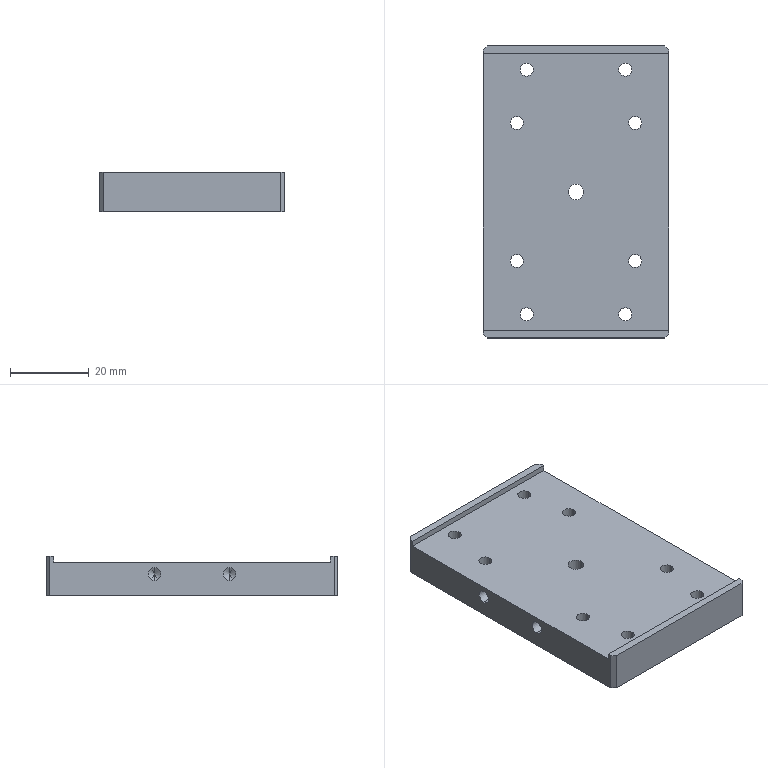Part | NX | features BREP 1 | 1 solid | 52 faces | box 47 x 74 x 10 mm | volume 28659 mm3 | cylinder 28 | plane 14 | cone 10 | commonest cylinder face diameters 3.3 x24 2.5 x2 4 x2
STEP:
#1=CARTESIAN_POINT('',(0.,22.5,5.25));
#2=VERTEX_POINT('',#1);
#3=CARTESIAN_POINT('',(0.,22.5,7.75));
#4=VERTEX_POINT('',#3);
#5=CARTESIAN_POINT('',(0.,22.5,6.5));
#6=DIRECTION('',(0.,1.,0.));
#7=DIRECTION('',(0.,0.,1.));
#8=AXIS2_PLACEMENT_3D('',#5,#6,#7);
#9=CIRCLE('',#8,1.25);
#10=EDGE_CURVE('',#2,#4,#9,.T.);
#11=ORIENTED_EDGE('',*,*,#10,.F.);
#12=CARTESIAN_POINT('',(0.,37.,5.25));
#13=VERTEX_POINT('',#12);
#14=CARTESIAN_POINT('',(0.,37.,5.25));
#15=DIRECTION('',(0.,1.,0.));
#16=VECTOR('',#15,1000.);
#17=LINE('',#14,#16);
#18=EDGE_CURVE('',#13,#2,#17,.F.);
#19=ORIENTED_EDGE('',*,*,#18,.F.);
#20=CARTESIAN_POINT('',(0.,37.,7.75));
#21=VERTEX_POINT('',#20);
#22=CARTESIAN_POINT('',(0.,37.,6.5));
#23=DIRECTION('',(0.,1.,0.));
#24=DIRECTION('',(0.,0.,1.));
#25=AXIS2_PLACEMENT_3D('',#22,#23,#24);
#26=CIRCLE('',#25,1.25);
#27=EDGE_CURVE('',#13,#21,#26,.T.);
#28=ORIENTED_EDGE('',*,*,#27,.T.);
#29=CARTESIAN_POINT('',(0.,37.,7.75));
#30=DIRECTION('',(0.,1.,0.));
#31=VECTOR('',#30,1000.);
#32=LINE('',#29,#31);
#33=EDGE_CURVE('',#21,#4,#32,.F.);
#34=ORIENTED_EDGE('',*,*,#33,.T.);
#35=EDGE_LOOP('',(#11,#19,#28,#34));
#36=FACE_BOUND('',#35,.T.);
#37=CARTESIAN_POINT('',(0.,37.,6.5));
#38=DIRECTION('',(0.,1.,0.));
#39=DIRECTION('',(0.,0.,1.));
#40=AXIS2_PLACEMENT_3D('',#37,#38,#39);
#41=CYLINDRICAL_SURFACE('',#40,1.25);
#42=ADVANCED_FACE('',(#36),#41,.F.);
#43=CARTESIAN_POINT('',(0.,21.749,6.5));
#44=VERTEX_POINT('',#43);
#45=CARTESIAN_POINT('',(0.,22.5,7.75));
#46=DIRECTION('',(0.,0.515,0.8572));
#47=VECTOR('',#46,1000.);
#48=LINE('',#45,#47);
#49=EDGE_CURVE('',#4,#44,#48,.F.);
#50=ORIENTED_EDGE('',*,*,#49,.T.);
#51=CARTESIAN_POINT('',(0.,22.5,5.25));
#52=DIRECTION('',(0.,0.515,-0.8572));
#53=VECTOR('',#52,1000.);
#54=LINE('',#51,#53);
#55=EDGE_CURVE('',#2,#44,#54,.F.);
#56=ORIENTED_EDGE('',*,*,#55,.F.);
#57=ORIENTED_EDGE('',*,*,#10,.T.);
#58=EDGE_LOOP('',(#50,#56,#57));
#59=FACE_BOUND('',#58,.T.);
#60=CARTESIAN_POINT('',(0.,22.5,6.5));
#61=DIRECTION('',(0.,1.,0.));
#62=DIRECTION('',(0.,0.,1.));
#63=AXIS2_PLACEMENT_3D('',#60,#61,#62);
#64=CONICAL_SURFACE('',#63,1.25,1.03);
#65=ADVANCED_FACE('',(#59),#64,.F.);
#66=CARTESIAN_POINT('',(12.,9.5,7.15));
#67=VERTEX_POINT('',#66);
#68=CARTESIAN_POINT('',(12.,9.5,3.85));
#69=VERTEX_POINT('',#68);
#70=CARTESIAN_POINT('',(12.,9.5,5.5));
#71=DIRECTION('',(1.,0.,0.));
#72=DIRECTION('',(0.,0.,-1.));
#73=AXIS2_PLACEMENT_3D('',#70,#71,#72);
#74=CIRCLE('',#73,1.65);
#75=EDGE_CURVE('',#67,#69,#74,.T.);
#76=ORIENTED_EDGE('',*,*,#75,.F.);
#77=CARTESIAN_POINT('',(23.5,9.5,7.15));
#78=VERTEX_POINT('',#77);
#79=CARTESIAN_POINT('',(23.5,9.5,7.15));
#80=DIRECTION('',(1.,0.,0.));
#81=VECTOR('',#80,1000.);
#82=LINE('',#79,#81);
#83=EDGE_CURVE('',#67,#78,#82,.T.);
#84=ORIENTED_EDGE('',*,*,#83,.T.);
#85=CARTESIAN_POINT('',(23.5,9.5,3.85));
#86=VERTEX_POINT('',#85);
#87=CARTESIAN_POINT('',(23.5,9.5,5.5));
#88=DIRECTION('',(1.,0.,0.));
#89=DIRECTION('',(0.,0.,-1.));
#90=AXIS2_PLACEMENT_3D('',#87,#88,#89);
#91=CIRCLE('',#90,1.65);
#92=EDGE_CURVE('',#78,#86,#91,.T.);
#93=ORIENTED_EDGE('',*,*,#92,.T.);
#94=CARTESIAN_POINT('',(23.5,9.5,3.85));
#95=DIRECTION('',(1.,0.,0.));
#96=VECTOR('',#95,1000.);
#97=LINE('',#94,#96);
#98=EDGE_CURVE('',#69,#86,#97,.T.);
#99=ORIENTED_EDGE('',*,*,#98,.F.);
#100=EDGE_LOOP('',(#76,#84,#93,#99));
#101=FACE_BOUND('',#100,.T.);
#102=CARTESIAN_POINT('',(23.5,9.5,5.5));
#103=DIRECTION('',(1.,0.,0.));
#104=DIRECTION('',(0.,0.,-1.));
#105=AXIS2_PLACEMENT_3D('',#102,#103,#104);
#106=CYLINDRICAL_SURFACE('',#105,1.65);
#107=ADVANCED_FACE('',(#101),#106,.F.);
#108=CARTESIAN_POINT('',(11.009,9.5,5.5));
#109=VERTEX_POINT('',#108);
#110=CARTESIAN_POINT('',(12.,9.5,3.85));
#111=DIRECTION('',(0.515,0.,-0.8572));
#112=VECTOR('',#111,1000.);
#113=LINE('',#110,#112);
#114=EDGE_CURVE('',#109,#69,#113,.T.);
#115=ORIENTED_EDGE('',*,*,#114,.F.);
#116=CARTESIAN_POINT('',(12.,9.5,7.15));
#117=DIRECTION('',(0.515,0.,0.8572));
#118=VECTOR('',#117,1000.);
#119=LINE('',#116,#118);
#120=EDGE_CURVE('',#109,#67,#119,.T.);
#121=ORIENTED_EDGE('',*,*,#120,.T.);
#122=ORIENTED_EDGE('',*,*,#75,.T.);
#123=EDGE_LOOP('',(#115,#121,#122));
#124=FACE_BOUND('',#123,.T.);
#125=CARTESIAN_POINT('',(12.,9.5,5.5));
#126=DIRECTION('',(1.,0.,0.));
#127=DIRECTION('',(0.,0.,-1.));
#128=AXIS2_PLACEMENT_3D('',#125,#126,#127);
#129=CONICAL_SURFACE('',#128,1.65,1.03);
#130=ADVANCED_FACE('',(#124),#129,.F.);
#131=CARTESIAN_POINT('',(12.,-9.5,7.15));
#132=VERTEX_POINT('',#131);
#133=CARTESIAN_POINT('',(12.,-9.5,3.85));
#134=VERTEX_POINT('',#133);
#135=CARTESIAN_POINT('',(12.,-9.5,5.5));
#136=DIRECTION('',(1.,0.,0.));
#137=DIRECTION('',(0.,0.,-1.));
#138=AXIS2_PLACEMENT_3D('',#135,#136,#137);
#139=CIRCLE('',#138,1.65);
#140=EDGE_CURVE('',#132,#134,#139,.T.);
#141=ORIENTED_EDGE('',*,*,#140,.F.);
#142=CARTESIAN_POINT('',(23.5,-9.5,7.15));
#143=VERTEX_POINT('',#142);
#144=CARTESIAN_POINT('',(23.5,-9.5,7.15));
#145=DIRECTION('',(1.,0.,0.));
#146=VECTOR('',#145,1000.);
#147=LINE('',#144,#146);
#148=EDGE_CURVE('',#132,#143,#147,.T.);
#149=ORIENTED_EDGE('',*,*,#148,.T.);
#150=CARTESIAN_POINT('',(23.5,-9.5,3.85));
#151=VERTEX_POINT('',#150);
#152=CARTESIAN_POINT('',(23.5,-9.5,5.5));
#153=DIRECTION('',(1.,0.,0.));
#154=DIRECTION('',(0.,0.,-1.));
#155=AXIS2_PLACEMENT_3D('',#152,#153,#154);
#156=CIRCLE('',#155,1.65);
#157=EDGE_CURVE('',#143,#151,#156,.T.);
#158=ORIENTED_EDGE('',*,*,#157,.T.);
#159=CARTESIAN_POINT('',(23.5,-9.5,3.85));
#160=DIRECTION('',(1.,0.,0.));
#161=VECTOR('',#160,1000.);
#162=LINE('',#159,#161);
#163=EDGE_CURVE('',#134,#151,#162,.T.);
#164=ORIENTED_EDGE('',*,*,#163,.F.);
#165=EDGE_LOOP('',(#141,#149,#158,#164));
#166=FACE_BOUND('',#165,.T.);
#167=CARTESIAN_POINT('',(23.5,-9.5,5.5));
#168=DIRECTION('',(1.,0.,0.));
#169=DIRECTION('',(0.,0.,-1.));
#170=AXIS2_PLACEMENT_3D('',#167,#168,#169);
#171=CYLINDRICAL_SURFACE('',#170,1.65);
#172=ADVANCED_FACE('',(#166),#171,.F.);
#173=CARTESIAN_POINT('',(11.009,-9.5,5.5));
#174=VERTEX_POINT('',#173);
#175=CARTESIAN_POINT('',(12.,-9.5,3.85));
#176=DIRECTION('',(0.515,0.,-0.8572));
#177=VECTOR('',#176,1000.);
#178=LINE('',#175,#177);
#179=EDGE_CURVE('',#174,#134,#178,.T.);
#180=ORIENTED_EDGE('',*,*,#179,.F.);
#181=CARTESIAN_POINT('',(12.,-9.5,7.15));
#182=DIRECTION('',(0.515,0.,0.8572));
#183=VECTOR('',#182,1000.);
#184=LINE('',#181,#183);
#185=EDGE_CURVE('',#174,#132,#184,.T.);
#186=ORIENTED_EDGE('',*,*,#185,.T.);
#187=ORIENTED_EDGE('',*,*,#140,.T.);
#188=EDGE_LOOP('',(#180,#186,#187));
#189=FACE_BOUND('',#188,.T.);
#190=CARTESIAN_POINT('',(12.,-9.5,5.5));
#191=DIRECTION('',(1.,0.,0.));
#192=DIRECTION('',(0.,0.,-1.));
#193=AXIS2_PLACEMENT_3D('',#190,#191,#192);
#194=CONICAL_SURFACE('',#193,1.65,1.03);
#195=ADVANCED_FACE('',(#189),#194,.F.);
#196=CARTESIAN_POINT('',(-12.,9.5,3.85));
#197=VERTEX_POINT('',#196);
#198=CARTESIAN_POINT('',(-12.,9.5,7.15));
#199=VERTEX_POINT('',#198);
#200=CARTESIAN_POINT('',(-12.,9.5,5.5));
#201=DIRECTION('',(-1.,0.,0.));
#202=DIRECTION('',(0.,0.,1.));
#203=AXIS2_PLACEMENT_3D('',#200,#201,#202);
#204=CIRCLE('',#203,1.65);
#205=EDGE_CURVE('',#197,#199,#204,.T.);
#206=ORIENTED_EDGE('',*,*,#205,.F.);
#207=CARTESIAN_POINT('',(-23.5,9.5,3.85));
#208=VERTEX_POINT('',#207);
#209=CARTESIAN_POINT('',(-23.5,9.5,3.85));
#210=DIRECTION('',(-1.,0.,0.));
#211=VECTOR('',#210,1000.);
#212=LINE('',#209,#211);
#213=EDGE_CURVE('',#208,#197,#212,.F.);
#214=ORIENTED_EDGE('',*,*,#213,.F.);
#215=CARTESIAN_POINT('',(-23.5,9.5,7.15));
#216=VERTEX_POINT('',#215);
#217=CARTESIAN_POINT('',(-23.5,9.5,5.5));
#218=DIRECTION('',(-1.,0.,0.));
#219=DIRECTION('',(0.,0.,1.));
#220=AXIS2_PLACEMENT_3D('',#217,#218,#219);
#221=CIRCLE('',#220,1.65);
#222=EDGE_CURVE('',#208,#216,#221,.T.);
#223=ORIENTED_EDGE('',*,*,#222,.T.);
#224=CARTESIAN_POINT('',(-23.5,9.5,7.15));
#225=DIRECTION('',(-1.,0.,0.));
#226=VECTOR('',#225,1000.);
#227=LINE('',#224,#226);
#228=EDGE_CURVE('',#216,#199,#227,.F.);
#229=ORIENTED_EDGE('',*,*,#228,.T.);
#230=EDGE_LOOP('',(#206,#214,#223,#229));
#231=FACE_BOUND('',#230,.T.);
#232=CARTESIAN_POINT('',(-23.5,9.5,5.5));
#233=DIRECTION('',(-1.,0.,0.));
#234=DIRECTION('',(0.,0.,1.));
#235=AXIS2_PLACEMENT_3D('',#232,#233,#234);
#236=CYLINDRICAL_SURFACE('',#235,1.65);
#237=ADVANCED_FACE('',(#231),#236,.F.);
#238=CARTESIAN_POINT('',(-11.009,9.5,5.5));
#239=VERTEX_POINT('',#238);
#240=CARTESIAN_POINT('',(-12.,9.5,7.15));
#241=DIRECTION('',(-0.515,0.,0.8572));
#242=VECTOR('',#241,1000.);
#243=LINE('',#240,#242);
#244=EDGE_CURVE('',#199,#239,#243,.F.);
#245=ORIENTED_EDGE('',*,*,#244,.T.);
#246=CARTESIAN_POINT('',(-12.,9.5,3.85));
#247=DIRECTION('',(-0.515,0.,-0.8572));
#248=VECTOR('',#247,1000.);
#249=LINE('',#246,#248);
#250=EDGE_CURVE('',#197,#239,#249,.F.);
#251=ORIENTED_EDGE('',*,*,#250,.F.);
#252=ORIENTED_EDGE('',*,*,#205,.T.);
#253=EDGE_LOOP('',(#245,#251,#252));
#254=FACE_BOUND('',#253,.T.);
#255=CARTESIAN_POINT('',(-12.,9.5,5.5));
#256=DIRECTION('',(-1.,0.,0.));
#257=DIRECTION('',(0.,0.,1.));
#258=AXIS2_PLACEMENT_3D('',#255,#256,#257);
#259=CONICAL_SURFACE('',#258,1.65,1.03);
#260=ADVANCED_FACE('',(#254),#259,.F.);
#261=CARTESIAN_POINT('',(-12.,-9.5,3.85));
#262=VERTEX_POINT('',#261);
#263=CARTESIAN_POINT('',(-12.,-9.5,7.15));
#264=VERTEX_POINT('',#263);
#265=CARTESIAN_POINT('',(-12.,-9.5,5.5));
#266=DIRECTION('',(-1.,0.,0.));
#267=DIRECTION('',(0.,0.,1.));
#268=AXIS2_PLACEMENT_3D('',#265,#266,#267);
#269=CIRCLE('',#268,1.65);
#270=EDGE_CURVE('',#262,#264,#269,.T.);
#271=ORIENTED_EDGE('',*,*,#270,.F.);
#272=CARTESIAN_POINT('',(-23.5,-9.5,3.85));
#273=VERTEX_POINT('',#272);
#274=CARTESIAN_POINT('',(-23.5,-9.5,3.85));
#275=DIRECTION('',(-1.,0.,0.));
#276=VECTOR('',#275,1000.);
#277=LINE('',#274,#276);
#278=EDGE_CURVE('',#273,#262,#277,.F.);
#279=ORIENTED_EDGE('',*,*,#278,.F.);
#280=CARTESIAN_POINT('',(-23.5,-9.5,7.15));
#281=VERTEX_POINT('',#280);
#282=CARTESIAN_POINT('',(-23.5,-9.5,5.5));
#283=DIRECTION('',(-1.,0.,0.));
#284=DIRECTION('',(0.,0.,1.));
#285=AXIS2_PLACEMENT_3D('',#282,#283,#284);
#286=CIRCLE('',#285,1.65);
#287=EDGE_CURVE('',#273,#281,#286,.T.);
#288=ORIENTED_EDGE('',*,*,#287,.T.);
#289=CARTESIAN_POINT('',(-23.5,-9.5,7.15));
#290=DIRECTION('',(-1.,0.,0.));
#291=VECTOR('',#290,1000.);
#292=LINE('',#289,#291);
#293=EDGE_CURVE('',#281,#264,#292,.F.);
#294=ORIENTED_EDGE('',*,*,#293,.T.);
#295=EDGE_LOOP('',(#271,#279,#288,#294));
#296=FACE_BOUND('',#295,.T.);
#297=CARTESIAN_POINT('',(-23.5,-9.5,5.5));
#298=DIRECTION('',(-1.,0.,0.));
#299=DIRECTION('',(0.,0.,1.));
#300=AXIS2_PLACEMENT_3D('',#297,#298,#299);
#301=CYLINDRICAL_SURFACE('',#300,1.65);
#302=ADVANCED_FACE('',(#296),#301,.F.);
#303=CARTESIAN_POINT('',(-11.009,-9.5,5.5));
#304=VERTEX_POINT('',#303);
#305=CARTESIAN_POINT('',(-12.,-9.5,7.15));
#306=DIRECTION('',(-0.515,0.,0.8572));
#307=VECTOR('',#306,1000.);
#308=LINE('',#305,#307);
#309=EDGE_CURVE('',#264,#304,#308,.F.);
#310=ORIENTED_EDGE('',*,*,#309,.T.);
#311=CARTESIAN_POINT('',(-12.,-9.5,3.85));
#312=DIRECTION('',(-0.515,0.,-0.8572));
#313=VECTOR('',#312,1000.);
#314=LINE('',#311,#313);
#315=EDGE_CURVE('',#262,#304,#314,.F.);
#316=ORIENTED_EDGE('',*,*,#315,.F.);
#317=ORIENTED_EDGE('',*,*,#270,.T.);
#318=EDGE_LOOP('',(#310,#316,#317));
#319=FACE_BOUND('',#318,.T.);
#320=CARTESIAN_POINT('',(-12.,-9.5,5.5));
#321=DIRECTION('',(-1.,0.,0.));
#322=DIRECTION('',(0.,0.,1.));
#323=AXIS2_PLACEMENT_3D('',#320,#321,#322);
#324=CONICAL_SURFACE('',#323,1.65,1.03);
#325=ADVANCED_FACE('',(#319),#324,.F.);
#326=CARTESIAN_POINT('',(13.35,17.5,8.5));
#327=VERTEX_POINT('',#326);
#328=CARTESIAN_POINT('',(16.65,17.5,8.5));
#329=VERTEX_POINT('',#328);
#330=CARTESIAN_POINT('',(15.,17.5,8.5));
#331=DIRECTION('',(0.,0.,1.));
#332=DIRECTION('',(1.,0.,0.));
#333=AXIS2_PLACEMENT_3D('',#330,#331,#332);
#334=CIRCLE('',#333,1.65);
#335=EDGE_CURVE('',#327,#329,#334,.T.);
#336=ORIENTED_EDGE('',*,*,#335,.T.);
#337=CARTESIAN_POINT('',(16.65,17.5,0.));
#338=VERTEX_POINT('',#337);
#339=CARTESIAN_POINT('',(16.65,17.5,0.));
#340=DIRECTION('',(0.,0.,-1.));
#341=VECTOR('',#340,1000.);
#342=LINE('',#339,#341);
#343=EDGE_CURVE('',#329,#338,#342,.T.);
#344=ORIENTED_EDGE('',*,*,#343,.T.);
#345=CARTESIAN_POINT('',(13.35,17.5,0.));
#346=VERTEX_POINT('',#345);
#347=CARTESIAN_POINT('',(15.,17.5,0.));
#348=DIRECTION('',(0.,0.,-1.));
#349=DIRECTION('',(-1.,0.,0.));
#350=AXIS2_PLACEMENT_3D('',#347,#348,#349);
#351=CIRCLE('',#350,1.65);
#352=EDGE_CURVE('',#338,#346,#351,.T.);
#353=ORIENTED_EDGE('',*,*,#352,.T.);
#354=CARTESIAN_POINT('',(13.35,17.5,0.));
#355=DIRECTION('',(0.,0.,-1.));
#356=VECTOR('',#355,1000.);
#357=LINE('',#354,#356);
#358=EDGE_CURVE('',#327,#346,#357,.T.);
#359=ORIENTED_EDGE('',*,*,#358,.F.);
#360=EDGE_LOOP('',(#336,#344,#353,#359));
#361=FACE_BOUND('',#360,.T.);
#362=CARTESIAN_POINT('',(15.,17.5,0.));
#363=DIRECTION('',(0.,0.,-1.));
#364=DIRECTION('',(-1.,0.,0.));
#365=AXIS2_PLACEMENT_3D('',#362,#363,#364);
#366=CYLINDRICAL_SURFACE('',#365,1.65);
#367=ADVANCED_FACE('',(#361),#366,.F.);
#368=CARTESIAN_POINT('',(13.35,-17.5,8.5));
#369=VERTEX_POINT('',#368);
#370=CARTESIAN_POINT('',(16.65,-17.5,8.5));
#371=VERTEX_POINT('',#370);
#372=CARTESIAN_POINT('',(15.,-17.5,8.5));
#373=DIRECTION('',(0.,0.,1.));
#374=DIRECTION('',(1.,0.,0.));
#375=AXIS2_PLACEMENT_3D('',#372,#373,#374);
#376=CIRCLE('',#375,1.65);
#377=EDGE_CURVE('',#369,#371,#376,.T.);
#378=ORIENTED_EDGE('',*,*,#377,.T.);
#379=CARTESIAN_POINT('',(16.65,-17.5,0.));
#380=VERTEX_POINT('',#379);
#381=CARTESIAN_POINT('',(16.65,-17.5,0.));
#382=DIRECTION('',(0.,0.,-1.));
#383=VECTOR('',#382,1000.);
#384=LINE('',#381,#383);
#385=EDGE_CURVE('',#371,#380,#384,.T.);
#386=ORIENTED_EDGE('',*,*,#385,.T.);
#387=CARTESIAN_POINT('',(13.35,-17.5,0.));
#388=VERTEX_POINT('',#387);
#389=CARTESIAN_POINT('',(15.,-17.5,0.));
#390=DIRECTION('',(0.,0.,-1.));
#391=DIRECTION('',(-1.,0.,0.));
#392=AXIS2_PLACEMENT_3D('',#389,#390,#391);
#393=CIRCLE('',#392,1.65);
#394=EDGE_CURVE('',#380,#388,#393,.T.);
#395=ORIENTED_EDGE('',*,*,#394,.T.);
#396=CARTESIAN_POINT('',(13.35,-17.5,0.));
#397=DIRECTION('',(0.,0.,-1.));
#398=VECTOR('',#397,1000.);
#399=LINE('',#396,#398);
#400=EDGE_CURVE('',#369,#388,#399,.T.);
#401=ORIENTED_EDGE('',*,*,#400,.F.);
#402=EDGE_LOOP('',(#378,#386,#395,#401));
#403=FACE_BOUND('',#402,.T.);
#404=CARTESIAN_POINT('',(15.,-17.5,0.));
#405=DIRECTION('',(0.,0.,-1.));
#406=DIRECTION('',(-1.,0.,0.));
#407=AXIS2_PLACEMENT_3D('',#404,#405,#406);
#408=CYLINDRICAL_SURFACE('',#407,1.65);
#409=ADVANCED_FACE('',(#403),#408,.F.);
#410=CARTESIAN_POINT('',(-16.65,17.5,8.5));
#411=VERTEX_POINT('',#410);
#412=CARTESIAN_POINT('',(-13.35,17.5,8.5));
#413=VERTEX_POINT('',#412);
#414=CARTESIAN_POINT('',(-15.,17.5,8.5));
#415=DIRECTION('',(0.,0.,1.));
#416=DIRECTION('',(1.,0.,0.));
#417=AXIS2_PLACEMENT_3D('',#414,#415,#416);
#418=CIRCLE('',#417,1.65);
#419=EDGE_CURVE('',#411,#413,#418,.T.);
#420=ORIENTED_EDGE('',*,*,#419,.T.);
#421=CARTESIAN_POINT('',(-13.35,17.5,0.));
#422=VERTEX_POINT('',#421);
#423=CARTESIAN_POINT('',(-13.35,17.5,0.));
#424=DIRECTION('',(0.,0.,-1.));
#425=VECTOR('',#424,1000.);
#426=LINE('',#423,#425);
#427=EDGE_CURVE('',#413,#422,#426,.T.);
#428=ORIENTED_EDGE('',*,*,#427,.T.);
#429=CARTESIAN_POINT('',(-16.65,17.5,0.));
#430=VERTEX_POINT('',#429);
#431=CARTESIAN_POINT('',(-15.,17.5,0.));
#432=DIRECTION('',(0.,0.,-1.));
#433=DIRECTION('',(-1.,0.,0.));
#434=AXIS2_PLACEMENT_3D('',#431,#432,#433);
#435=CIRCLE('',#434,1.65);
#436=EDGE_CURVE('',#422,#430,#435,.T.);
#437=ORIENTED_EDGE('',*,*,#436,.T.);
#438=CARTESIAN_POINT('',(-16.65,17.5,0.));
#439=DIRECTION('',(0.,0.,-1.));
#440=VECTOR('',#439,1000.);
#441=LINE('',#438,#440);
#442=EDGE_CURVE('',#411,#430,#441,.T.);
#443=ORIENTED_EDGE('',*,*,#442,.F.);
#444=EDGE_LOOP('',(#420,#428,#437,#443));
#445=FACE_BOUND('',#444,.T.);
#446=CARTESIAN_POINT('',(-15.,17.5,0.));
#447=DIRECTION('',(0.,0.,-1.));
#448=DIRECTION('',(-1.,0.,0.));
#449=AXIS2_PLACEMENT_3D('',#446,#447,#448);
#450=CYLINDRICAL_SURFACE('',#449,1.65);
#451=ADVANCED_FACE('',(#445),#450,.F.);
#452=CARTESIAN_POINT('',(-16.65,-17.5,8.5));
#453=VERTEX_POINT('',#452);
#454=CARTESIAN_POINT('',(-13.35,-17.5,8.5));
#455=VERTEX_POINT('',#454);
#456=CARTESIAN_POINT('',(-15.,-17.5,8.5));
#457=DIRECTION('',(0.,0.,1.));
#458=DIRECTION('',(1.,0.,0.));
#459=AXIS2_PLACEMENT_3D('',#456,#457,#458);
#460=CIRCLE('',#459,1.65);
#461=EDGE_CURVE('',#453,#455,#460,.T.);
#462=ORIENTED_EDGE('',*,*,#461,.T.);
#463=CARTESIAN_POINT('',(-13.35,-17.5,0.));
#464=VERTEX_POINT('',#463);
#465=CARTESIAN_POINT('',(-13.35,-17.5,0.));
#466=DIRECTION('',(0.,0.,-1.));
#467=VECTOR('',#466,1000.);
#468=LINE('',#465,#467);
#469=EDGE_CURVE('',#455,#464,#468,.T.);
#470=ORIENTED_EDGE('',*,*,#469,.T.);
#471=CARTESIAN_POINT('',(-16.65,-17.5,0.));
#472=VERTEX_POINT('',#471);
#473=CARTESIAN_POINT('',(-15.,-17.5,0.));
#474=DIRECTION('',(0.,0.,-1.));
#475=DIRECTION('',(-1.,0.,0.));
#476=AXIS2_PLACEMENT_3D('',#473,#474,#475);
#477=CIRCLE('',#476,1.65);
#478=EDGE_CURVE('',#464,#472,#477,.T.);
#479=ORIENTED_EDGE('',*,*,#478,.T.);
#480=CARTESIAN_POINT('',(-16.65,-17.5,0.));
#481=DIRECTION('',(0.,0.,-1.));
#482=VECTOR('',#481,1000.);
#483=LINE('',#480,#482);
#484=EDGE_CURVE('',#453,#472,#483,.T.);
#485=ORIENTED_EDGE('',*,*,#484,.F.);
#486=EDGE_LOOP('',(#462,#470,#479,#485));
#487=FACE_BOUND('',#486,.T.);
#488=CARTESIAN_POINT('',(-15.,-17.5,0.));
#489=DIRECTION('',(0.,0.,-1.));
#490=DIRECTION('',(-1.,0.,0.));
#491=AXIS2_PLACEMENT_3D('',#488,#489,#490);
#492=CYLINDRICAL_SURFACE('',#491,1.65);
#493=ADVANCED_FACE('',(#487),#492,.F.);
#494=CARTESIAN_POINT('',(-14.15,-31.,0.));
#495=VERTEX_POINT('',#494);
#496=CARTESIAN_POINT('',(-10.85,-31.,0.));
#497=VERTEX_POINT('',#496);
#498=CARTESIAN_POINT('',(-12.5,-31.,0.));
#499=DIRECTION('',(0.,0.,1.));
#500=DIRECTION('',(1.,0.,0.));
#501=AXIS2_PLACEMENT_3D('',#498,#499,#500);
#502=CIRCLE('',#501,1.65);
#503=EDGE_CURVE('',#495,#497,#502,.T.);
#504=ORIENTED_EDGE('',*,*,#503,.F.);
#505=CARTESIAN_POINT('',(-14.15,-31.,8.5));
#506=VERTEX_POINT('',#505);
#507=CARTESIAN_POINT('',(-14.15,-31.,8.5));
#508=DIRECTION('',(0.,0.,1.));
#509=VECTOR('',#508,1000.);
#510=LINE('',#507,#509);
#511=EDGE_CURVE('',#506,#495,#510,.F.);
#512=ORIENTED_EDGE('',*,*,#511,.F.);
#513=CARTESIAN_POINT('',(-10.85,-31.,8.5));
#514=VERTEX_POINT('',#513);
#515=CARTESIAN_POINT('',(-12.5,-31.,8.5));
#516=DIRECTION('',(0.,0.,1.));
#517=DIRECTION('',(1.,0.,0.));
#518=AXIS2_PLACEMENT_3D('',#515,#516,#517);
#519=CIRCLE('',#518,1.65);
#520=EDGE_CURVE('',#506,#514,#519,.T.);
#521=ORIENTED_EDGE('',*,*,#520,.T.);
#522=CARTESIAN_POINT('',(-10.85,-31.,8.5));
#523=DIRECTION('',(0.,0.,1.));
#524=VECTOR('',#523,1000.);
#525=LINE('',#522,#524);
#526=EDGE_CURVE('',#514,#497,#525,.F.);
#527=ORIENTED_EDGE('',*,*,#526,.T.);
#528=EDGE_LOOP('',(#504,#512,#521,#527));
#529=FACE_BOUND('',#528,.T.);
#530=CARTESIAN_POINT('',(-12.5,-31.,8.5));
#531=DIRECTION('',(0.,0.,1.));
#532=DIRECTION('',(1.,0.,0.));
#533=AXIS2_PLACEMENT_3D('',#530,#531,#532);
#534=CYLINDRICAL_SURFACE('',#533,1.65);
#535=ADVANCED_FACE('',(#529),#534,.F.);
#536=CARTESIAN_POINT('',(10.85,-31.,0.));
#537=VERTEX_POINT('',#536);
#538=CARTESIAN_POINT('',(14.15,-31.,0.));
#539=VERTEX_POINT('',#538);
#540=CARTESIAN_POINT('',(12.5,-31.,0.));
#541=DIRECTION('',(0.,0.,1.));
#542=DIRECTION('',(1.,0.,0.));
#543=AXIS2_PLACEMENT_3D('',#540,#541,#542);
#544=CIRCLE('',#543,1.65);
#545=EDGE_CURVE('',#537,#539,#544,.T.);
#546=ORIENTED_EDGE('',*,*,#545,.F.);
#547=CARTESIAN_POINT('',(10.85,-31.,8.5));
#548=VERTEX_POINT('',#547);
#549=CARTESIAN_POINT('',(10.85,-31.,8.5));
#550=DIRECTION('',(0.,0.,1.));
#551=VECTOR('',#550,1000.);
#552=LINE('',#549,#551);
#553=EDGE_CURVE('',#548,#537,#552,.F.);
#554=ORIENTED_EDGE('',*,*,#553,.F.);
#555=CARTESIAN_POINT('',(14.15,-31.,8.5));
#556=VERTEX_POINT('',#555);
#557=CARTESIAN_POINT('',(12.5,-31.,8.5));
#558=DIRECTION('',(0.,0.,1.));
#559=DIRECTION('',(1.,0.,0.));
#560=AXIS2_PLACEMENT_3D('',#557,#558,#559);
#561=CIRCLE('',#560,1.65);
#562=EDGE_CURVE('',#548,#556,#561,.T.);
#563=ORIENTED_EDGE('',*,*,#562,.T.);
#564=CARTESIAN_POINT('',(14.15,-31.,8.5));
#565=DIRECTION('',(0.,0.,1.));
#566=VECTOR('',#565,1000.);
#567=LINE('',#564,#566);
#568=EDGE_CURVE('',#556,#539,#567,.F.);
#569=ORIENTED_EDGE('',*,*,#568,.T.);
#570=EDGE_LOOP('',(#546,#554,#563,#569));
#571=FACE_BOUND('',#570,.T.);
#572=CARTESIAN_POINT('',(12.5,-31.,8.5));
#573=DIRECTION('',(0.,0.,1.));
#574=DIRECTION('',(1.,0.,0.));
#575=AXIS2_PLACEMENT_3D('',#572,#573,#574);
#576=CYLINDRICAL_SURFACE('',#575,1.65);
#577=ADVANCED_FACE('',(#571),#576,.F.);
#578=CARTESIAN_POINT('',(-14.15,31.,0.));
#579=VERTEX_POINT('',#578);
#580=CARTESIAN_POINT('',(-10.85,31.,0.));
#581=VERTEX_POINT('',#580);
#582=CARTESIAN_POINT('',(-12.5,31.,0.));
#583=DIRECTION('',(0.,0.,1.));
#584=DIRECTION('',(1.,0.,0.));
#585=AXIS2_PLACEMENT_3D('',#582,#583,#584);
#586=CIRCLE('',#585,1.65);
#587=EDGE_CURVE('',#579,#581,#586,.T.);
#588=ORIENTED_EDGE('',*,*,#587,.F.);
#589=CARTESIAN_POINT('',(-14.15,31.,8.5));
#590=VERTEX_POINT('',#589);
#591=CARTESIAN_POINT('',(-14.15,31.,8.5));
#592=DIRECTION('',(0.,0.,1.));
#593=VECTOR('',#592,1000.);
#594=LINE('',#591,#593);
#595=EDGE_CURVE('',#590,#579,#594,.F.);
#596=ORIENTED_EDGE('',*,*,#595,.F.);
#597=CARTESIAN_POINT('',(-10.85,31.,8.5));
#598=VERTEX_POINT('',#597);
#599=CARTESIAN_POINT('',(-12.5,31.,8.5));
#600=DIRECTION('',(0.,0.,1.));
#601=DIRECTION('',(1.,0.,0.));
#602=AXIS2_PLACEMENT_3D('',#599,#600,#601);
#603=CIRCLE('',#602,1.65);
#604=EDGE_CURVE('',#590,#598,#603,.T.);
#605=ORIENTED_EDGE('',*,*,#604,.T.);
#606=CARTESIAN_POINT('',(-10.85,31.,8.5));
#607=DIRECTION('',(0.,0.,1.));
#608=VECTOR('',#607,1000.);
#609=LINE('',#606,#608);
#610=EDGE_CURVE('',#598,#581,#609,.F.);
#611=ORIENTED_EDGE('',*,*,#610,.T.);
#612=EDGE_LOOP('',(#588,#596,#605,#611));
#613=FACE_BOUND('',#612,.T.);
#614=CARTESIAN_POINT('',(-12.5,31.,8.5));
#615=DIRECTION('',(0.,0.,1.));
#616=DIRECTION('',(1.,0.,0.));
#617=AXIS2_PLACEMENT_3D('',#614,#615,#616);
#618=CYLINDRICAL_SURFACE('',#617,1.65);
#619=ADVANCED_FACE('',(#613),#618,.F.);
#620=CARTESIAN_POINT('',(10.85,31.,0.));
#621=VERTEX_POINT('',#620);
#622=CARTESIAN_POINT('',(14.15,31.,0.));
#623=VERTEX_POINT('',#622);
#624=CARTESIAN_POINT('',(12.5,31.,0.));
#625=DIRECTION('',(0.,0.,1.));
#626=DIRECTION('',(1.,0.,0.));
#627=AXIS2_PLACEMENT_3D('',#624,#625,#626);
#628=CIRCLE('',#627,1.65);
#629=EDGE_CURVE('',#621,#623,#628,.T.);
#630=ORIENTED_EDGE('',*,*,#629,.F.);
#631=CARTESIAN_POINT('',(10.85,31.,8.5));
#632=VERTEX_POINT('',#631);
#633=CARTESIAN_POINT('',(10.85,31.,8.5));
#634=DIRECTION('',(0.,0.,1.));
#635=VECTOR('',#634,1000.);
#636=LINE('',#633,#635);
#637=EDGE_CURVE('',#632,#621,#636,.F.);
#638=ORIENTED_EDGE('',*,*,#637,.F.);
#639=CARTESIAN_POINT('',(14.15,31.,8.5));
#640=VERTEX_POINT('',#639);
#641=CARTESIAN_POINT('',(12.5,31.,8.5));
#642=DIRECTION('',(0.,0.,1.));
#643=DIRECTION('',(1.,0.,0.));
#644=AXIS2_PLACEMENT_3D('',#641,#642,#643);
#645=CIRCLE('',#644,1.65);
#646=EDGE_CURVE('',#632,#640,#645,.T.);
#647=ORIENTED_EDGE('',*,*,#646,.T.);
#648=CARTESIAN_POINT('',(14.15,31.,8.5));
#649=DIRECTION('',(0.,0.,1.));
#650=VECTOR('',#649,1000.);
#651=LINE('',#648,#650);
#652=EDGE_CURVE('',#640,#623,#651,.F.);
#653=ORIENTED_EDGE('',*,*,#652,.T.);
#654=EDGE_LOOP('',(#630,#638,#647,#653));
#655=FACE_BOUND('',#654,.T.);
#656=CARTESIAN_POINT('',(12.5,31.,8.5));
#657=DIRECTION('',(0.,0.,1.));
#658=DIRECTION('',(1.,0.,0.));
#659=AXIS2_PLACEMENT_3D('',#656,#657,#658);
#660=CYLINDRICAL_SURFACE('',#659,1.65);
#661=ADVANCED_FACE('',(#655),#660,.F.);
#662=CARTESIAN_POINT('',(-2.,0.,0.));
#663=VERTEX_POINT('',#662);
#664=CARTESIAN_POINT('',(2.,0.,0.));
#665=VERTEX_POINT('',#664);
#666=CARTESIAN_POINT('',(0.,0.,0.));
#667=DIRECTION('',(0.,0.,1.));
#668=DIRECTION('',(1.,0.,0.));
#669=AXIS2_PLACEMENT_3D('',#666,#667,#668);
#670=CIRCLE('',#669,2.);
#671=EDGE_CURVE('',#663,#665,#670,.T.);
#672=ORIENTED_EDGE('',*,*,#671,.F.);
#673=CARTESIAN_POINT('',(-2.,0.,8.5));
#674=VERTEX_POINT('',#673);
#675=CARTESIAN_POINT('',(-2.,0.,0.));
#676=DIRECTION('',(0.,0.,1.));
#677=VECTOR('',#676,1000.);
#678=LINE('',#675,#677);
#679=EDGE_CURVE('',#674,#663,#678,.F.);
#680=ORIENTED_EDGE('',*,*,#679,.F.);
#681=CARTESIAN_POINT('',(2.,0.,8.5));
#682=VERTEX_POINT('',#681);
#683=CARTESIAN_POINT('',(0.,0.,8.5));
#684=DIRECTION('',(0.,0.,-1.));
#685=DIRECTION('',(1.,0.,0.));
#686=AXIS2_PLACEMENT_3D('',#683,#684,#685);
#687=CIRCLE('',#686,2.);
#688=EDGE_CURVE('',#682,#674,#687,.T.);
#689=ORIENTED_EDGE('',*,*,#688,.F.);
#690=CARTESIAN_POINT('',(2.,0.,0.));
#691=DIRECTION('',(0.,0.,1.));
#692=VECTOR('',#691,1000.);
#693=LINE('',#690,#692);
#694=EDGE_CURVE('',#682,#665,#693,.F.);
#695=ORIENTED_EDGE('',*,*,#694,.T.);
#696=EDGE_LOOP('',(#672,#680,#689,#695));
#697=FACE_BOUND('',#696,.T.);
#698=CARTESIAN_POINT('',(0.,0.,0.));
#699=DIRECTION('',(0.,0.,1.));
#700=DIRECTION('',(1.,0.,0.));
#701=AXIS2_PLACEMENT_3D('',#698,#699,#700);
#702=CYLINDRICAL_SURFACE('',#701,2.);
#703=ADVANCED_FACE('',(#697),#702,.F.);
#704=CARTESIAN_POINT('',(-23.5,-35.,10.));
#705=VERTEX_POINT('',#704);
#706=CARTESIAN_POINT('',(-23.5,-36.,10.));
#707=VERTEX_POINT('',#706);
#708=CARTESIAN_POINT('',(-23.5,37.,10.));
#709=DIRECTION('',(0.,-1.,0.));
#710=VECTOR('',#709,1000.);
#711=LINE('',#708,#710);
#712=EDGE_CURVE('',#705,#707,#711,.T.);
#713=ORIENTED_EDGE('',*,*,#712,.T.);
#714=CARTESIAN_POINT('',(-22.5,-37.,10.));
#715=VERTEX_POINT('',#714);
#716=CARTESIAN_POINT('',(-29.75,-29.75,10.));
#717=DIRECTION('',(0.7071,-0.7071,0.));
#718=VECTOR('',#717,1000.);
#719=LINE('',#716,#718);
#720=EDGE_CURVE('',#707,#715,#719,.T.);
#721=ORIENTED_EDGE('',*,*,#720,.T.);
#722=CARTESIAN_POINT('',(22.5,-37.,10.));
#723=VERTEX_POINT('',#722);
#724=CARTESIAN_POINT('',(-23.5,-37.,10.));
#725=DIRECTION('',(1.,0.,0.));
#726=VECTOR('',#725,1000.);
#727=LINE('',#724,#726);
#728=EDGE_CURVE('',#715,#723,#727,.T.);
#729=ORIENTED_EDGE('',*,*,#728,.T.);
#730=CARTESIAN_POINT('',(23.5,-36.,10.));
#731=VERTEX_POINT('',#730);
#732=CARTESIAN_POINT('',(29.75,-29.75,10.));
#733=DIRECTION('',(0.7071,0.7071,0.));
#734=VECTOR('',#733,1000.);
#735=LINE('',#732,#734);
#736=EDGE_CURVE('',#723,#731,#735,.T.);
#737=ORIENTED_EDGE('',*,*,#736,.T.);
#738=CARTESIAN_POINT('',(23.5,-35.,10.));
#739=VERTEX_POINT('',#738);
#740=CARTESIAN_POINT('',(23.5,37.,10.));
#741=DIRECTION('',(0.,1.,0.));
#742=VECTOR('',#741,1000.);
#743=LINE('',#740,#742);
#744=EDGE_CURVE('',#731,#739,#743,.T.);
#745=ORIENTED_EDGE('',*,*,#744,.T.);
#746=CARTESIAN_POINT('',(-23.5,-35.,10.));
#747=DIRECTION('',(1.,0.,0.));
#748=VECTOR('',#747,1000.);
#749=LINE('',#746,#748);
#750=EDGE_CURVE('',#705,#739,#749,.T.);
#751=ORIENTED_EDGE('',*,*,#750,.F.);
#752=EDGE_LOOP('',(#713,#721,#729,#737,#745,#751));
#753=FACE_BOUND('',#752,.T.);
#754=CARTESIAN_POINT('',(0.,0.,10.));
#755=DIRECTION('',(0.,0.,1.));
#756=DIRECTION('',(1.,0.,0.));
#757=AXIS2_PLACEMENT_3D('',#754,#755,#756);
#758=PLANE('',#757);
#759=ADVANCED_FACE('',(#753),#758,.T.);
#760=ORIENTED_EDGE('',*,*,#679,.T.);
#761=CARTESIAN_POINT('',(0.,0.,0.));
#762=DIRECTION('',(0.,0.,1.));
#763=DIRECTION('',(1.,0.,0.));
#764=AXIS2_PLACEMENT_3D('',#761,#762,#763);
#765=CIRCLE('',#764,2.);
#766=EDGE_CURVE('',#665,#663,#765,.T.);
#767=ORIENTED_EDGE('',*,*,#766,.F.);
#768=ORIENTED_EDGE('',*,*,#694,.F.);
#769=CARTESIAN_POINT('',(0.,0.,8.5));
#770=DIRECTION('',(0.,0.,-1.));
#771=DIRECTION('',(1.,0.,0.));
#772=AXIS2_PLACEMENT_3D('',#769,#770,#771);
#773=CIRCLE('',#772,2.);
#774=EDGE_CURVE('',#674,#682,#773,.T.);
#775=ORIENTED_EDGE('',*,*,#774,.F.);
#776=EDGE_LOOP('',(#760,#767,#768,#775));
#777=FACE_BOUND('',#776,.T.);
#778=CARTESIAN_POINT('',(0.,0.,0.));
#779=DIRECTION('',(0.,0.,1.));
#780=DIRECTION('',(1.,0.,0.));
#781=AXIS2_PLACEMENT_3D('',#778,#779,#780);
#782=CYLINDRICAL_SURFACE('',#781,2.);
#783=ADVANCED_FACE('',(#777),#782,.F.);
#784=ORIENTED_EDGE('',*,*,#744,.F.);
#785=CARTESIAN_POINT('',(23.5,-36.,0.));
#786=VERTEX_POINT('',#785);
#787=CARTESIAN_POINT('',(23.5,-36.,10.));
#788=DIRECTION('',(0.,0.,-1.));
#789=VECTOR('',#788,1000.);
#790=LINE('',#787,#789);
#791=EDGE_CURVE('',#731,#786,#790,.T.);
#792=ORIENTED_EDGE('',*,*,#791,.T.);
#793=CARTESIAN_POINT('',(23.5,36.,0.));
#794=VERTEX_POINT('',#793);
#795=CARTESIAN_POINT('',(23.5,37.,0.));
#796=DIRECTION('',(0.,1.,0.));
#797=VECTOR('',#796,1000.);
#798=LINE('',#795,#797);
#799=EDGE_CURVE('',#786,#794,#798,.T.);
#800=ORIENTED_EDGE('',*,*,#799,.T.);
#801=CARTESIAN_POINT('',(23.5,36.,10.));
#802=VERTEX_POINT('',#801);
#803=CARTESIAN_POINT('',(23.5,36.,10.));
#804=DIRECTION('',(0.,0.,1.));
#805=VECTOR('',#804,1000.);
#806=LINE('',#803,#805);
#807=EDGE_CURVE('',#794,#802,#806,.T.);
#808=ORIENTED_EDGE('',*,*,#807,.T.);
#809=CARTESIAN_POINT('',(23.5,35.,10.));
#810=VERTEX_POINT('',#809);
#811=CARTESIAN_POINT('',(23.5,37.,10.));
#812=DIRECTION('',(0.,1.,0.));
#813=VECTOR('',#812,1000.);
#814=LINE('',#811,#813);
#815=EDGE_CURVE('',#810,#802,#814,.T.);
#816=ORIENTED_EDGE('',*,*,#815,.F.);
#817=CARTESIAN_POINT('',(23.5,35.,8.5));
#818=VERTEX_POINT('',#817);
#819=CARTESIAN_POINT('',(23.5,35.,8.5));
#820=DIRECTION('',(0.,0.,1.));
#821=VECTOR('',#820,1000.);
#822=LINE('',#819,#821);
#823=EDGE_CURVE('',#818,#810,#822,.T.);
#824=ORIENTED_EDGE('',*,*,#823,.F.);
#825=CARTESIAN_POINT('',(23.5,-35.,8.5));
#826=VERTEX_POINT('',#825);
#827=CARTESIAN_POINT('',(23.5,35.,8.5));
#828=DIRECTION('',(0.,1.,0.));
#829=VECTOR('',#828,1000.);
#830=LINE('',#827,#829);
#831=EDGE_CURVE('',#826,#818,#830,.T.);
#832=ORIENTED_EDGE('',*,*,#831,.F.);
#833=CARTESIAN_POINT('',(23.5,-35.,8.5));
#834=DIRECTION('',(0.,0.,1.));
#835=VECTOR('',#834,1000.);
#836=LINE('',#833,#835);
#837=EDGE_CURVE('',#826,#739,#836,.T.);
#838=ORIENTED_EDGE('',*,*,#837,.T.);
#839=EDGE_LOOP('',(#784,#792,#800,#808,#816,#824,#832,#838));
#840=FACE_BOUND('',#839,.T.);
#841=CARTESIAN_POINT('',(23.5,9.5,5.5));
#842=DIRECTION('',(1.,0.,0.));
#843=DIRECTION('',(0.,0.,-1.));
#844=AXIS2_PLACEMENT_3D('',#841,#842,#843);
#845=CIRCLE('',#844,1.65);
#846=EDGE_CURVE('',#86,#78,#845,.T.);
#847=ORIENTED_EDGE('',*,*,#846,.F.);
#848=ORIENTED_EDGE('',*,*,#92,.F.);
#849=EDGE_LOOP('',(#847,#848));
#850=FACE_BOUND('',#849,.T.);
#851=CARTESIAN_POINT('',(23.5,-9.5,5.5));
#852=DIRECTION('',(1.,0.,0.));
#853=DIRECTION('',(0.,0.,-1.));
#854=AXIS2_PLACEMENT_3D('',#851,#852,#853);
#855=CIRCLE('',#854,1.65);
#856=EDGE_CURVE('',#151,#143,#855,.T.);
#857=ORIENTED_EDGE('',*,*,#856,.F.);
#858=ORIENTED_EDGE('',*,*,#157,.F.);
#859=EDGE_LOOP('',(#857,#858));
#860=FACE_BOUND('',#859,.T.);
#861=CARTESIAN_POINT('',(23.5,37.,10.));
#862=DIRECTION('',(-1.,0.,0.));
#863=DIRECTION('',(0.,1.,0.));
#864=AXIS2_PLACEMENT_3D('',#861,#862,#863);
#865=PLANE('',#864);
#866=ADVANCED_FACE('',(#840,#850,#860),#865,.F.);
#867=CARTESIAN_POINT('',(22.5,37.,10.));
#868=VERTEX_POINT('',#867);
#869=CARTESIAN_POINT('',(-22.5,37.,10.));
#870=VERTEX_POINT('',#869);
#871=CARTESIAN_POINT('',(-23.5,37.,10.));
#872=DIRECTION('',(-1.,0.,0.));
#873=VECTOR('',#872,1000.);
#874=LINE('',#871,#873);
#875=EDGE_CURVE('',#868,#870,#874,.T.);
#876=ORIENTED_EDGE('',*,*,#875,.F.);
#877=CARTESIAN_POINT('',(22.5,37.,0.));
#878=VERTEX_POINT('',#877);
#879=CARTESIAN_POINT('',(22.5,37.,10.));
#880=DIRECTION('',(0.,0.,-1.));
#881=VECTOR('',#880,1000.);
#882=LINE('',#879,#881);
#883=EDGE_CURVE('',#868,#878,#882,.T.);
#884=ORIENTED_EDGE('',*,*,#883,.T.);
#885=CARTESIAN_POINT('',(-22.5,37.,0.));
#886=VERTEX_POINT('',#885);
#887=CARTESIAN_POINT('',(-23.5,37.,0.));
#888=DIRECTION('',(-1.,0.,0.));
#889=VECTOR('',#888,1000.);
#890=LINE('',#887,#889);
#891=EDGE_CURVE('',#878,#886,#890,.T.);
#892=ORIENTED_EDGE('',*,*,#891,.T.);
#893=CARTESIAN_POINT('',(-22.5,37.,10.));
#894=DIRECTION('',(0.,0.,1.));
#895=VECTOR('',#894,1000.);
#896=LINE('',#893,#895);
#897=EDGE_CURVE('',#886,#870,#896,.T.);
#898=ORIENTED_EDGE('',*,*,#897,.T.);
#899=EDGE_LOOP('',(#876,#884,#892,#898));
#900=FACE_BOUND('',#899,.T.);
#901=CARTESIAN_POINT('',(0.,37.,6.5));
#902=DIRECTION('',(0.,1.,0.));
#903=DIRECTION('',(0.,0.,1.));
#904=AXIS2_PLACEMENT_3D('',#901,#902,#903);
#905=CIRCLE('',#904,1.25);
#906=EDGE_CURVE('',#21,#13,#905,.T.);
#907=ORIENTED_EDGE('',*,*,#906,.F.);
#908=ORIENTED_EDGE('',*,*,#27,.F.);
#909=EDGE_LOOP('',(#907,#908));
#910=FACE_BOUND('',#909,.T.);
#911=CARTESIAN_POINT('',(-23.5,37.,10.));
#912=DIRECTION('',(0.,-1.,0.));
#913=DIRECTION('',(0.,0.,-1.));
#914=AXIS2_PLACEMENT_3D('',#911,#912,#913);
#915=PLANE('',#914);
#916=ADVANCED_FACE('',(#900,#910),#915,.F.);
#917=CARTESIAN_POINT('',(-23.5,36.,0.));
#918=VERTEX_POINT('',#917);
#919=CARTESIAN_POINT('',(-23.5,-36.,0.));
#920=VERTEX_POINT('',#919);
#921=CARTESIAN_POINT('',(-23.5,37.,0.));
#922=DIRECTION('',(0.,-1.,0.));
#923=VECTOR('',#922,1000.);
#924=LINE('',#921,#923);
#925=EDGE_CURVE('',#918,#920,#924,.T.);
#926=ORIENTED_EDGE('',*,*,#925,.T.);
#927=CARTESIAN_POINT('',(-23.5,-36.,10.));
#928=DIRECTION('',(0.,0.,1.));
#929=VECTOR('',#928,1000.);
#930=LINE('',#927,#929);
#931=EDGE_CURVE('',#920,#707,#930,.T.);
#932=ORIENTED_EDGE('',*,*,#931,.T.);
#933=ORIENTED_EDGE('',*,*,#712,.F.);
#934=CARTESIAN_POINT('',(-23.5,-35.,8.5));
#935=VERTEX_POINT('',#934);
#936=CARTESIAN_POINT('',(-23.5,-35.,8.5));
#937=DIRECTION('',(0.,0.,1.));
#938=VECTOR('',#937,1000.);
#939=LINE('',#936,#938);
#940=EDGE_CURVE('',#935,#705,#939,.T.);
#941=ORIENTED_EDGE('',*,*,#940,.F.);
#942=CARTESIAN_POINT('',(-23.5,35.,8.5));
#943=VERTEX_POINT('',#942);
#944=CARTESIAN_POINT('',(-23.5,35.,8.5));
#945=DIRECTION('',(0.,-1.,0.));
#946=VECTOR('',#945,1000.);
#947=LINE('',#944,#946);
#948=EDGE_CURVE('',#943,#935,#947,.T.);
#949=ORIENTED_EDGE('',*,*,#948,.F.);
#950=CARTESIAN_POINT('',(-23.5,35.,10.));
#951=VERTEX_POINT('',#950);
#952=CARTESIAN_POINT('',(-23.5,35.,8.5));
#953=DIRECTION('',(0.,0.,1.));
#954=VECTOR('',#953,1000.);
#955=LINE('',#952,#954);
#956=EDGE_CURVE('',#943,#951,#955,.T.);
#957=ORIENTED_EDGE('',*,*,#956,.T.);
#958=CARTESIAN_POINT('',(-23.5,36.,10.));
#959=VERTEX_POINT('',#958);
#960=CARTESIAN_POINT('',(-23.5,37.,10.));
#961=DIRECTION('',(0.,-1.,0.));
#962=VECTOR('',#961,1000.);
#963=LINE('',#960,#962);
#964=EDGE_CURVE('',#959,#951,#963,.T.);
#965=ORIENTED_EDGE('',*,*,#964,.F.);
#966=CARTESIAN_POINT('',(-23.5,36.,10.));
#967=DIRECTION('',(0.,0.,-1.));
#968=VECTOR('',#967,1000.);
#969=LINE('',#966,#968);
#970=EDGE_CURVE('',#959,#918,#969,.T.);
#971=ORIENTED_EDGE('',*,*,#970,.T.);
#972=EDGE_LOOP('',(#926,#932,#933,#941,#949,#957,#965,#971));
#973=FACE_BOUND('',#972,.T.);
#974=CARTESIAN_POINT('',(-23.5,9.5,5.5));
#975=DIRECTION('',(-1.,0.,0.));
#976=DIRECTION('',(0.,0.,1.));
#977=AXIS2_PLACEMENT_3D('',#974,#975,#976);
#978=CIRCLE('',#977,1.65);
#979=EDGE_CURVE('',#216,#208,#978,.T.);
#980=ORIENTED_EDGE('',*,*,#979,.F.);
#981=ORIENTED_EDGE('',*,*,#222,.F.);
#982=EDGE_LOOP('',(#980,#981));
#983=FACE_BOUND('',#982,.T.);
#984=CARTESIAN_POINT('',(-23.5,-9.5,5.5));
#985=DIRECTION('',(-1.,0.,0.));
#986=DIRECTION('',(0.,0.,1.));
#987=AXIS2_PLACEMENT_3D('',#984,#985,#986);
#988=CIRCLE('',#987,1.65);
#989=EDGE_CURVE('',#281,#273,#988,.T.);
#990=ORIENTED_EDGE('',*,*,#989,.F.);
#991=ORIENTED_EDGE('',*,*,#287,.F.);
#992=EDGE_LOOP('',(#990,#991));
#993=FACE_BOUND('',#992,.T.);
#994=CARTESIAN_POINT('',(-23.5,37.,10.));
#995=DIRECTION('',(1.,0.,0.));
#996=DIRECTION('',(0.,1.,0.));
#997=AXIS2_PLACEMENT_3D('',#994,#995,#996);
#998=PLANE('',#997);
#999=ADVANCED_FACE('',(#973,#983,#993),#998,.F.);
#1000=ORIENTED_EDGE('',*,*,#728,.F.);
#1001=CARTESIAN_POINT('',(-22.5,-37.,0.));
#1002=VERTEX_POINT('',#1001);
#1003=CARTESIAN_POINT('',(-22.5,-37.,10.));
#1004=DIRECTION('',(0.,0.,-1.));
#1005=VECTOR('',#1004,1000.);
#1006=LINE('',#1003,#1005);
#1007=EDGE_CURVE('',#715,#1002,#1006,.T.);
#1008=ORIENTED_EDGE('',*,*,#1007,.T.);
#1009=CARTESIAN_POINT('',(22.5,-37.,0.));
#1010=VERTEX_POINT('',#1009);
#1011=CARTESIAN_POINT('',(-23.5,-37.,0.));
#1012=DIRECTION('',(1.,0.,0.));
#1013=VECTOR('',#1012,1000.);
#1014=LINE('',#1011,#1013);
#1015=EDGE_CURVE('',#1002,#1010,#1014,.T.);
#1016=ORIENTED_EDGE('',*,*,#1015,.T.);
#1017=CARTESIAN_POINT('',(22.5,-37.,10.));
#1018=DIRECTION('',(0.,0.,1.));
#1019=VECTOR('',#1018,1000.);
#1020=LINE('',#1017,#1019);
#1021=EDGE_CURVE('',#1010,#723,#1020,.T.);
#1022=ORIENTED_EDGE('',*,*,#1021,.T.);
#1023=EDGE_LOOP('',(#1000,#1008,#1016,#1022));
#1024=FACE_BOUND('',#1023,.T.);
#1025=CARTESIAN_POINT('',(-23.5,-37.,10.));
#1026=DIRECTION('',(0.,1.,0.));
#1027=DIRECTION('',(1.,0.,0.));
#1028=AXIS2_PLACEMENT_3D('',#1025,#1026,#1027);
#1029=PLANE('',#1028);
#1030=ADVANCED_FACE('',(#1024),#1029,.F.);
#1031=ORIENTED_EDGE('',*,*,#815,.T.);
#1032=CARTESIAN_POINT('',(29.75,29.75,10.));
#1033=DIRECTION('',(-0.7071,0.7071,0.));
#1034=VECTOR('',#1033,1000.);
#1035=LINE('',#1032,#1034);
#1036=EDGE_CURVE('',#802,#868,#1035,.T.);
#1037=ORIENTED_EDGE('',*,*,#1036,.T.);
#1038=ORIENTED_EDGE('',*,*,#875,.T.);
#1039=CARTESIAN_POINT('',(-29.75,29.75,10.));
#1040=DIRECTION('',(-0.7071,-0.7071,0.));
#1041=VECTOR('',#1040,1000.);
#1042=LINE('',#1039,#1041);
#1043=EDGE_CURVE('',#870,#959,#1042,.T.);
#1044=ORIENTED_EDGE('',*,*,#1043,.T.);
#1045=ORIENTED_EDGE('',*,*,#964,.T.);
#1046=CARTESIAN_POINT('',(-23.5,35.,10.));
#1047=DIRECTION('',(-1.,0.,0.));
#1048=VECTOR('',#1047,1000.);
#1049=LINE('',#1046,#1048);
#1050=EDGE_CURVE('',#810,#951,#1049,.T.);
#1051=ORIENTED_EDGE('',*,*,#1050,.F.);
#1052=EDGE_LOOP('',(#1031,#1037,#1038,#1044,#1045,#1051));
#1053=FACE_BOUND('',#1052,.T.);
#1054=CARTESIAN_POINT('',(0.,0.,10.));
#1055=DIRECTION('',(0.,0.,1.));
#1056=DIRECTION('',(1.,0.,0.));
#1057=AXIS2_PLACEMENT_3D('',#1054,#1055,#1056);
#1058=PLANE('',#1057);
#1059=ADVANCED_FACE('',(#1053),#1058,.T.);
#1060=ORIENTED_EDGE('',*,*,#1015,.F.);
#1061=CARTESIAN_POINT('',(-22.5,-37.,0.));
#1062=DIRECTION('',(-0.7071,0.7071,0.));
#1063=VECTOR('',#1062,1000.);
#1064=LINE('',#1061,#1063);
#1065=EDGE_CURVE('',#1002,#920,#1064,.T.);
#1066=ORIENTED_EDGE('',*,*,#1065,.T.);
#1067=ORIENTED_EDGE('',*,*,#925,.F.);
#1068=CARTESIAN_POINT('',(-23.5,36.,0.));
#1069=DIRECTION('',(0.7071,0.7071,0.));
#1070=VECTOR('',#1069,1000.);
#1071=LINE('',#1068,#1070);
#1072=EDGE_CURVE('',#918,#886,#1071,.T.);
#1073=ORIENTED_EDGE('',*,*,#1072,.T.);
#1074=ORIENTED_EDGE('',*,*,#891,.F.);
#1075=CARTESIAN_POINT('',(22.5,37.,0.));
#1076=DIRECTION('',(0.7071,-0.7071,0.));
#1077=VECTOR('',#1076,1000.);
#1078=LINE('',#1075,#1077);
#1079=EDGE_CURVE('',#878,#794,#1078,.T.);
#1080=ORIENTED_EDGE('',*,*,#1079,.T.);
#1081=ORIENTED_EDGE('',*,*,#799,.F.);
#1082=CARTESIAN_POINT('',(23.5,-36.,0.));
#1083=DIRECTION('',(-0.7071,-0.7071,0.));
#1084=VECTOR('',#1083,1000.);
#1085=LINE('',#1082,#1084);
#1086=EDGE_CURVE('',#786,#1010,#1085,.T.);
#1087=ORIENTED_EDGE('',*,*,#1086,.T.);
#1088=EDGE_LOOP('',(#1060,#1066,#1067,#1073,#1074,#1080,#1081,#1087));
#1089=FACE_BOUND('',#1088,.T.);
#1090=CARTESIAN_POINT('',(15.,17.5,0.));
#1091=DIRECTION('',(0.,0.,-1.));
#1092=DIRECTION('',(-1.,0.,0.));
#1093=AXIS2_PLACEMENT_3D('',#1090,#1091,#1092);
#1094=CIRCLE('',#1093,1.65);
#1095=EDGE_CURVE('',#346,#338,#1094,.T.);
#1096=ORIENTED_EDGE('',*,*,#1095,.F.);
#1097=ORIENTED_EDGE('',*,*,#352,.F.);
#1098=EDGE_LOOP('',(#1096,#1097));
#1099=FACE_BOUND('',#1098,.T.);
#1100=CARTESIAN_POINT('',(15.,-17.5,0.));
#1101=DIRECTION('',(0.,0.,-1.));
#1102=DIRECTION('',(-1.,0.,0.));
#1103=AXIS2_PLACEMENT_3D('',#1100,#1101,#1102);
#1104=CIRCLE('',#1103,1.65);
#1105=EDGE_CURVE('',#388,#380,#1104,.T.);
#1106=ORIENTED_EDGE('',*,*,#1105,.F.);
#1107=ORIENTED_EDGE('',*,*,#394,.F.);
#1108=EDGE_LOOP('',(#1106,#1107));
#1109=FACE_BOUND('',#1108,.T.);
#1110=CARTESIAN_POINT('',(-15.,17.5,0.));
#1111=DIRECTION('',(0.,0.,-1.));
#1112=DIRECTION('',(-1.,0.,0.));
#1113=AXIS2_PLACEMENT_3D('',#1110,#1111,#1112);
#1114=CIRCLE('',#1113,1.65);
#1115=EDGE_CURVE('',#430,#422,#1114,.T.);
#1116=ORIENTED_EDGE('',*,*,#1115,.F.);
#1117=ORIENTED_EDGE('',*,*,#436,.F.);
#1118=EDGE_LOOP('',(#1116,#1117));
#1119=FACE_BOUND('',#1118,.T.);
#1120=CARTESIAN_POINT('',(-15.,-17.5,0.));
#1121=DIRECTION('',(0.,0.,-1.));
#1122=DIRECTION('',(-1.,0.,0.));
#1123=AXIS2_PLACEMENT_3D('',#1120,#1121,#1122);
#1124=CIRCLE('',#1123,1.65);
#1125=EDGE_CURVE('',#472,#464,#1124,.T.);
#1126=ORIENTED_EDGE('',*,*,#1125,.F.);
#1127=ORIENTED_EDGE('',*,*,#478,.F.);
#1128=EDGE_LOOP('',(#1126,#1127));
#1129=FACE_BOUND('',#1128,.T.);
#1130=CARTESIAN_POINT('',(-12.5,-31.,0.));
#1131=DIRECTION('',(0.,0.,1.));
#1132=DIRECTION('',(1.,0.,0.));
#1133=AXIS2_PLACEMENT_3D('',#1130,#1131,#1132);
#1134=CIRCLE('',#1133,1.65);
#1135=EDGE_CURVE('',#497,#495,#1134,.T.);
#1136=ORIENTED_EDGE('',*,*,#1135,.T.);
#1137=ORIENTED_EDGE('',*,*,#503,.T.);
#1138=EDGE_LOOP('',(#1136,#1137));
#1139=FACE_BOUND('',#1138,.T.);
#1140=CARTESIAN_POINT('',(12.5,-31.,0.));
#1141=DIRECTION('',(0.,0.,1.));
#1142=DIRECTION('',(1.,0.,0.));
#1143=AXIS2_PLACEMENT_3D('',#1140,#1141,#1142);
#1144=CIRCLE('',#1143,1.65);
#1145=EDGE_CURVE('',#539,#537,#1144,.T.);
#1146=ORIENTED_EDGE('',*,*,#1145,.T.);
#1147=ORIENTED_EDGE('',*,*,#545,.T.);
#1148=EDGE_LOOP('',(#1146,#1147));
#1149=FACE_BOUND('',#1148,.T.);
#1150=CARTESIAN_POINT('',(-12.5,31.,0.));
#1151=DIRECTION('',(0.,0.,1.));
#1152=DIRECTION('',(1.,0.,0.));
#1153=AXIS2_PLACEMENT_3D('',#1150,#1151,#1152);
#1154=CIRCLE('',#1153,1.65);
#1155=EDGE_CURVE('',#581,#579,#1154,.T.);
#1156=ORIENTED_EDGE('',*,*,#1155,.T.);
#1157=ORIENTED_EDGE('',*,*,#587,.T.);
#1158=EDGE_LOOP('',(#1156,#1157));
#1159=FACE_BOUND('',#1158,.T.);
#1160=CARTESIAN_POINT('',(12.5,31.,0.));
#1161=DIRECTION('',(0.,0.,1.));
#1162=DIRECTION('',(1.,0.,0.));
#1163=AXIS2_PLACEMENT_3D('',#1160,#1161,#1162);
#1164=CIRCLE('',#1163,1.65);
#1165=EDGE_CURVE('',#623,#621,#1164,.T.);
#1166=ORIENTED_EDGE('',*,*,#1165,.T.);
#1167=ORIENTED_EDGE('',*,*,#629,.T.);
#1168=EDGE_LOOP('',(#1166,#1167));
#1169=FACE_BOUND('',#1168,.T.);
#1170=ORIENTED_EDGE('',*,*,#766,.T.);
#1171=ORIENTED_EDGE('',*,*,#671,.T.);
#1172=EDGE_LOOP('',(#1170,#1171));
#1173=FACE_BOUND('',#1172,.T.);
#1174=CARTESIAN_POINT('',(0.,0.,0.));
#1175=DIRECTION('',(0.,0.,1.));
#1176=DIRECTION('',(1.,0.,0.));
#1177=AXIS2_PLACEMENT_3D('',#1174,#1175,#1176);
#1178=PLANE('',#1177);
#1179=ADVANCED_FACE('',(#1089,#1099,#1109,#1119,#1129,#1139,#1149,#1159,#1169,#1173),#1178,.F.);
#1180=ORIENTED_EDGE('',*,*,#831,.T.);
#1181=CARTESIAN_POINT('',(-23.5,35.,8.5));
#1182=DIRECTION('',(-1.,0.,0.));
#1183=VECTOR('',#1182,1000.);
#1184=LINE('',#1181,#1183);
#1185=EDGE_CURVE('',#818,#943,#1184,.T.);
#1186=ORIENTED_EDGE('',*,*,#1185,.T.);
#1187=ORIENTED_EDGE('',*,*,#948,.T.);
#1188=CARTESIAN_POINT('',(-23.5,-35.,8.5));
#1189=DIRECTION('',(1.,0.,0.));
#1190=VECTOR('',#1189,1000.);
#1191=LINE('',#1188,#1190);
#1192=EDGE_CURVE('',#935,#826,#1191,.T.);
#1193=ORIENTED_EDGE('',*,*,#1192,.T.);
#1194=EDGE_LOOP('',(#1180,#1186,#1187,#1193));
#1195=FACE_BOUND('',#1194,.T.);
#1196=ORIENTED_EDGE('',*,*,#335,.F.);
#1197=CARTESIAN_POINT('',(15.,17.5,8.5));
#1198=DIRECTION('',(0.,0.,1.));
#1199=DIRECTION('',(1.,0.,0.));
#1200=AXIS2_PLACEMENT_3D('',#1197,#1198,#1199);
#1201=CIRCLE('',#1200,1.65);
#1202=EDGE_CURVE('',#329,#327,#1201,.T.);
#1203=ORIENTED_EDGE('',*,*,#1202,.F.);
#1204=EDGE_LOOP('',(#1196,#1203));
#1205=FACE_BOUND('',#1204,.T.);
#1206=ORIENTED_EDGE('',*,*,#377,.F.);
#1207=CARTESIAN_POINT('',(15.,-17.5,8.5));
#1208=DIRECTION('',(0.,0.,1.));
#1209=DIRECTION('',(1.,0.,0.));
#1210=AXIS2_PLACEMENT_3D('',#1207,#1208,#1209);
#1211=CIRCLE('',#1210,1.65);
#1212=EDGE_CURVE('',#371,#369,#1211,.T.);
#1213=ORIENTED_EDGE('',*,*,#1212,.F.);
#1214=EDGE_LOOP('',(#1206,#1213));
#1215=FACE_BOUND('',#1214,.T.);
#1216=ORIENTED_EDGE('',*,*,#419,.F.);
#1217=CARTESIAN_POINT('',(-15.,17.5,8.5));
#1218=DIRECTION('',(0.,0.,1.));
#1219=DIRECTION('',(1.,0.,0.));
#1220=AXIS2_PLACEMENT_3D('',#1217,#1218,#1219);
#1221=CIRCLE('',#1220,1.65);
#1222=EDGE_CURVE('',#413,#411,#1221,.T.);
#1223=ORIENTED_EDGE('',*,*,#1222,.F.);
#1224=EDGE_LOOP('',(#1216,#1223));
#1225=FACE_BOUND('',#1224,.T.);
#1226=ORIENTED_EDGE('',*,*,#461,.F.);
#1227=CARTESIAN_POINT('',(-15.,-17.5,8.5));
#1228=DIRECTION('',(0.,0.,1.));
#1229=DIRECTION('',(1.,0.,0.));
#1230=AXIS2_PLACEMENT_3D('',#1227,#1228,#1229);
#1231=CIRCLE('',#1230,1.65);
#1232=EDGE_CURVE('',#455,#453,#1231,.T.);
#1233=ORIENTED_EDGE('',*,*,#1232,.F.);
#1234=EDGE_LOOP('',(#1226,#1233));
#1235=FACE_BOUND('',#1234,.T.);
#1236=CARTESIAN_POINT('',(-12.5,-31.,8.5));
#1237=DIRECTION('',(0.,0.,1.));
#1238=DIRECTION('',(1.,0.,0.));
#1239=AXIS2_PLACEMENT_3D('',#1236,#1237,#1238);
#1240=CIRCLE('',#1239,1.65);
#1241=EDGE_CURVE('',#514,#506,#1240,.T.);
#1242=ORIENTED_EDGE('',*,*,#1241,.F.);
#1243=ORIENTED_EDGE('',*,*,#520,.F.);
#1244=EDGE_LOOP('',(#1242,#1243));
#1245=FACE_BOUND('',#1244,.T.);
#1246=CARTESIAN_POINT('',(12.5,-31.,8.5));
#1247=DIRECTION('',(0.,0.,1.));
#1248=DIRECTION('',(1.,0.,0.));
#1249=AXIS2_PLACEMENT_3D('',#1246,#1247,#1248);
#1250=CIRCLE('',#1249,1.65);
#1251=EDGE_CURVE('',#556,#548,#1250,.T.);
#1252=ORIENTED_EDGE('',*,*,#1251,.F.);
#1253=ORIENTED_EDGE('',*,*,#562,.F.);
#1254=EDGE_LOOP('',(#1252,#1253));
#1255=FACE_BOUND('',#1254,.T.);
#1256=CARTESIAN_POINT('',(-12.5,31.,8.5));
#1257=DIRECTION('',(0.,0.,1.));
#1258=DIRECTION('',(1.,0.,0.));
#1259=AXIS2_PLACEMENT_3D('',#1256,#1257,#1258);
#1260=CIRCLE('',#1259,1.65);
#1261=EDGE_CURVE('',#598,#590,#1260,.T.);
#1262=ORIENTED_EDGE('',*,*,#1261,.F.);
#1263=ORIENTED_EDGE('',*,*,#604,.F.);
#1264=EDGE_LOOP('',(#1262,#1263));
#1265=FACE_BOUND('',#1264,.T.);
#1266=CARTESIAN_POINT('',(12.5,31.,8.5));
#1267=DIRECTION('',(0.,0.,1.));
#1268=DIRECTION('',(1.,0.,0.));
#1269=AXIS2_PLACEMENT_3D('',#1266,#1267,#1268);
#1270=CIRCLE('',#1269,1.65);
#1271=EDGE_CURVE('',#640,#632,#1270,.T.);
#1272=ORIENTED_EDGE('',*,*,#1271,.F.);
#1273=ORIENTED_EDGE('',*,*,#646,.F.);
#1274=EDGE_LOOP('',(#1272,#1273));
#1275=FACE_BOUND('',#1274,.T.);
#1276=ORIENTED_EDGE('',*,*,#688,.T.);
#1277=ORIENTED_EDGE('',*,*,#774,.T.);
#1278=EDGE_LOOP('',(#1276,#1277));
#1279=FACE_BOUND('',#1278,.T.);
#1280=CARTESIAN_POINT('',(0.,0.,8.5));
#1281=DIRECTION('',(0.,0.,1.));
#1282=DIRECTION('',(1.,0.,0.));
#1283=AXIS2_PLACEMENT_3D('',#1280,#1281,#1282);
#1284=PLANE('',#1283);
#1285=ADVANCED_FACE('',(#1195,#1205,#1215,#1225,#1235,#1245,#1255,#1265,#1275,#1279),#1284,.T.);
#1286=ORIENTED_EDGE('',*,*,#750,.T.);
#1287=ORIENTED_EDGE('',*,*,#837,.F.);
#1288=ORIENTED_EDGE('',*,*,#1192,.F.);
#1289=ORIENTED_EDGE('',*,*,#940,.T.);
#1290=EDGE_LOOP('',(#1286,#1287,#1288,#1289));
#1291=FACE_BOUND('',#1290,.T.);
#1292=CARTESIAN_POINT('',(-23.5,-35.,8.5));
#1293=DIRECTION('',(0.,-1.,0.));
#1294=DIRECTION('',(0.,0.,-1.));
#1295=AXIS2_PLACEMENT_3D('',#1292,#1293,#1294);
#1296=PLANE('',#1295);
#1297=ADVANCED_FACE('',(#1291),#1296,.F.);
#1298=ORIENTED_EDGE('',*,*,#1050,.T.);
#1299=ORIENTED_EDGE('',*,*,#956,.F.);
#1300=ORIENTED_EDGE('',*,*,#1185,.F.);
#1301=ORIENTED_EDGE('',*,*,#823,.T.);
#1302=EDGE_LOOP('',(#1298,#1299,#1300,#1301));
#1303=FACE_BOUND('',#1302,.T.);
#1304=CARTESIAN_POINT('',(-23.5,35.,8.5));
#1305=DIRECTION('',(0.,1.,0.));
#1306=DIRECTION('',(1.,0.,0.));
#1307=AXIS2_PLACEMENT_3D('',#1304,#1305,#1306);
#1308=PLANE('',#1307);
#1309=ADVANCED_FACE('',(#1303),#1308,.F.);
#1310=ORIENTED_EDGE('',*,*,#720,.F.);
#1311=ORIENTED_EDGE('',*,*,#931,.F.);
#1312=ORIENTED_EDGE('',*,*,#1065,.F.);
#1313=ORIENTED_EDGE('',*,*,#1007,.F.);
#1314=EDGE_LOOP('',(#1310,#1311,#1312,#1313));
#1315=FACE_BOUND('',#1314,.T.);
#1316=CARTESIAN_POINT('',(-22.5,-37.,10.));
#1317=DIRECTION('',(0.7071,0.7071,0.));
#1318=DIRECTION('',(0.,0.,-1.));
#1319=AXIS2_PLACEMENT_3D('',#1316,#1317,#1318);
#1320=PLANE('',#1319);
#1321=ADVANCED_FACE('',(#1315),#1320,.F.);
#1322=ORIENTED_EDGE('',*,*,#736,.F.);
#1323=ORIENTED_EDGE('',*,*,#1021,.F.);
#1324=ORIENTED_EDGE('',*,*,#1086,.F.);
#1325=ORIENTED_EDGE('',*,*,#791,.F.);
#1326=EDGE_LOOP('',(#1322,#1323,#1324,#1325));
#1327=FACE_BOUND('',#1326,.T.);
#1328=CARTESIAN_POINT('',(23.5,-36.,10.));
#1329=DIRECTION('',(-0.7071,0.7071,0.));
#1330=DIRECTION('',(0.,0.,1.));
#1331=AXIS2_PLACEMENT_3D('',#1328,#1329,#1330);
#1332=PLANE('',#1331);
#1333=ADVANCED_FACE('',(#1327),#1332,.F.);
#1334=ORIENTED_EDGE('',*,*,#1036,.F.);
#1335=ORIENTED_EDGE('',*,*,#807,.F.);
#1336=ORIENTED_EDGE('',*,*,#1079,.F.);
#1337=ORIENTED_EDGE('',*,*,#883,.F.);
#1338=EDGE_LOOP('',(#1334,#1335,#1336,#1337));
#1339=FACE_BOUND('',#1338,.T.);
#1340=CARTESIAN_POINT('',(22.5,37.,10.));
#1341=DIRECTION('',(-0.7071,-0.7071,0.));
#1342=DIRECTION('',(-0.7071,0.7071,0.));
#1343=AXIS2_PLACEMENT_3D('',#1340,#1341,#1342);
#1344=PLANE('',#1343);
#1345=ADVANCED_FACE('',(#1339),#1344,.F.);
#1346=ORIENTED_EDGE('',*,*,#1043,.F.);
#1347=ORIENTED_EDGE('',*,*,#897,.F.);
#1348=ORIENTED_EDGE('',*,*,#1072,.F.);
#1349=ORIENTED_EDGE('',*,*,#970,.F.);
#1350=EDGE_LOOP('',(#1346,#1347,#1348,#1349));
#1351=FACE_BOUND('',#1350,.T.);
#1352=CARTESIAN_POINT('',(-23.5,36.,10.));
#1353=DIRECTION('',(0.7071,-0.7071,0.));
#1354=DIRECTION('',(0.,0.,-1.));
#1355=AXIS2_PLACEMENT_3D('',#1352,#1353,#1354);
#1356=PLANE('',#1355);
#1357=ADVANCED_FACE('',(#1351),#1356,.F.);
#1358=ORIENTED_EDGE('',*,*,#637,.T.);
#1359=ORIENTED_EDGE('',*,*,#1165,.F.);
#1360=ORIENTED_EDGE('',*,*,#652,.F.);
#1361=ORIENTED_EDGE('',*,*,#1271,.T.);
#1362=EDGE_LOOP('',(#1358,#1359,#1360,#1361));
#1363=FACE_BOUND('',#1362,.T.);
#1364=CARTESIAN_POINT('',(12.5,31.,8.5));
#1365=DIRECTION('',(0.,0.,1.));
#1366=DIRECTION('',(1.,0.,0.));
#1367=AXIS2_PLACEMENT_3D('',#1364,#1365,#1366);
#1368=CYLINDRICAL_SURFACE('',#1367,1.65);
#1369=ADVANCED_FACE('',(#1363),#1368,.F.);
#1370=ORIENTED_EDGE('',*,*,#595,.T.);
#1371=ORIENTED_EDGE('',*,*,#1155,.F.);
#1372=ORIENTED_EDGE('',*,*,#610,.F.);
#1373=ORIENTED_EDGE('',*,*,#1261,.T.);
#1374=EDGE_LOOP('',(#1370,#1371,#1372,#1373));
#1375=FACE_BOUND('',#1374,.T.);
#1376=CARTESIAN_POINT('',(-12.5,31.,8.5));
#1377=DIRECTION('',(0.,0.,1.));
#1378=DIRECTION('',(1.,0.,0.));
#1379=AXIS2_PLACEMENT_3D('',#1376,#1377,#1378);
#1380=CYLINDRICAL_SURFACE('',#1379,1.65);
#1381=ADVANCED_FACE('',(#1375),#1380,.F.);
#1382=ORIENTED_EDGE('',*,*,#553,.T.);
#1383=ORIENTED_EDGE('',*,*,#1145,.F.);
#1384=ORIENTED_EDGE('',*,*,#568,.F.);
#1385=ORIENTED_EDGE('',*,*,#1251,.T.);
#1386=EDGE_LOOP('',(#1382,#1383,#1384,#1385));
#1387=FACE_BOUND('',#1386,.T.);
#1388=CARTESIAN_POINT('',(12.5,-31.,8.5));
#1389=DIRECTION('',(0.,0.,1.));
#1390=DIRECTION('',(1.,0.,0.));
#1391=AXIS2_PLACEMENT_3D('',#1388,#1389,#1390);
#1392=CYLINDRICAL_SURFACE('',#1391,1.65);
#1393=ADVANCED_FACE('',(#1387),#1392,.F.);
#1394=ORIENTED_EDGE('',*,*,#511,.T.);
#1395=ORIENTED_EDGE('',*,*,#1135,.F.);
#1396=ORIENTED_EDGE('',*,*,#526,.F.);
#1397=ORIENTED_EDGE('',*,*,#1241,.T.);
#1398=EDGE_LOOP('',(#1394,#1395,#1396,#1397));
#1399=FACE_BOUND('',#1398,.T.);
#1400=CARTESIAN_POINT('',(-12.5,-31.,8.5));
#1401=DIRECTION('',(0.,0.,1.));
#1402=DIRECTION('',(1.,0.,0.));
#1403=AXIS2_PLACEMENT_3D('',#1400,#1401,#1402);
#1404=CYLINDRICAL_SURFACE('',#1403,1.65);
#1405=ADVANCED_FACE('',(#1399),#1404,.F.);
#1406=ORIENTED_EDGE('',*,*,#469,.F.);
#1407=ORIENTED_EDGE('',*,*,#1232,.T.);
#1408=ORIENTED_EDGE('',*,*,#484,.T.);
#1409=ORIENTED_EDGE('',*,*,#1125,.T.);
#1410=EDGE_LOOP('',(#1406,#1407,#1408,#1409));
#1411=FACE_BOUND('',#1410,.T.);
#1412=CARTESIAN_POINT('',(-15.,-17.5,0.));
#1413=DIRECTION('',(0.,0.,-1.));
#1414=DIRECTION('',(-1.,0.,0.));
#1415=AXIS2_PLACEMENT_3D('',#1412,#1413,#1414);
#1416=CYLINDRICAL_SURFACE('',#1415,1.65);
#1417=ADVANCED_FACE('',(#1411),#1416,.F.);
#1418=ORIENTED_EDGE('',*,*,#427,.F.);
#1419=ORIENTED_EDGE('',*,*,#1222,.T.);
#1420=ORIENTED_EDGE('',*,*,#442,.T.);
#1421=ORIENTED_EDGE('',*,*,#1115,.T.);
#1422=EDGE_LOOP('',(#1418,#1419,#1420,#1421));
#1423=FACE_BOUND('',#1422,.T.);
#1424=CARTESIAN_POINT('',(-15.,17.5,0.));
#1425=DIRECTION('',(0.,0.,-1.));
#1426=DIRECTION('',(-1.,0.,0.));
#1427=AXIS2_PLACEMENT_3D('',#1424,#1425,#1426);
#1428=CYLINDRICAL_SURFACE('',#1427,1.65);
#1429=ADVANCED_FACE('',(#1423),#1428,.F.);
#1430=ORIENTED_EDGE('',*,*,#385,.F.);
#1431=ORIENTED_EDGE('',*,*,#1212,.T.);
#1432=ORIENTED_EDGE('',*,*,#400,.T.);
#1433=ORIENTED_EDGE('',*,*,#1105,.T.);
#1434=EDGE_LOOP('',(#1430,#1431,#1432,#1433));
#1435=FACE_BOUND('',#1434,.T.);
#1436=CARTESIAN_POINT('',(15.,-17.5,0.));
#1437=DIRECTION('',(0.,0.,-1.));
#1438=DIRECTION('',(-1.,0.,0.));
#1439=AXIS2_PLACEMENT_3D('',#1436,#1437,#1438);
#1440=CYLINDRICAL_SURFACE('',#1439,1.65);
#1441=ADVANCED_FACE('',(#1435),#1440,.F.);
#1442=ORIENTED_EDGE('',*,*,#343,.F.);
#1443=ORIENTED_EDGE('',*,*,#1202,.T.);
#1444=ORIENTED_EDGE('',*,*,#358,.T.);
#1445=ORIENTED_EDGE('',*,*,#1095,.T.);
#1446=EDGE_LOOP('',(#1442,#1443,#1444,#1445));
#1447=FACE_BOUND('',#1446,.T.);
#1448=CARTESIAN_POINT('',(15.,17.5,0.));
#1449=DIRECTION('',(0.,0.,-1.));
#1450=DIRECTION('',(-1.,0.,0.));
#1451=AXIS2_PLACEMENT_3D('',#1448,#1449,#1450);
#1452=CYLINDRICAL_SURFACE('',#1451,1.65);
#1453=ADVANCED_FACE('',(#1447),#1452,.F.);
#1454=ORIENTED_EDGE('',*,*,#315,.T.);
#1455=ORIENTED_EDGE('',*,*,#309,.F.);
#1456=CARTESIAN_POINT('',(-12.,-9.5,5.5));
#1457=DIRECTION('',(-1.,0.,0.));
#1458=DIRECTION('',(0.,0.,1.));
#1459=AXIS2_PLACEMENT_3D('',#1456,#1457,#1458);
#1460=CIRCLE('',#1459,1.65);
#1461=EDGE_CURVE('',#264,#262,#1460,.T.);
#1462=ORIENTED_EDGE('',*,*,#1461,.T.);
#1463=EDGE_LOOP('',(#1454,#1455,#1462));
#1464=FACE_BOUND('',#1463,.T.);
#1465=CARTESIAN_POINT('',(-12.,-9.5,5.5));
#1466=DIRECTION('',(-1.,0.,0.));
#1467=DIRECTION('',(0.,0.,1.));
#1468=AXIS2_PLACEMENT_3D('',#1465,#1466,#1467);
#1469=CONICAL_SURFACE('',#1468,1.65,1.03);
#1470=ADVANCED_FACE('',(#1464),#1469,.F.);
#1471=ORIENTED_EDGE('',*,*,#278,.T.);
#1472=ORIENTED_EDGE('',*,*,#1461,.F.);
#1473=ORIENTED_EDGE('',*,*,#293,.F.);
#1474=ORIENTED_EDGE('',*,*,#989,.T.);
#1475=EDGE_LOOP('',(#1471,#1472,#1473,#1474));
#1476=FACE_BOUND('',#1475,.T.);
#1477=CARTESIAN_POINT('',(-23.5,-9.5,5.5));
#1478=DIRECTION('',(-1.,0.,0.));
#1479=DIRECTION('',(0.,0.,1.));
#1480=AXIS2_PLACEMENT_3D('',#1477,#1478,#1479);
#1481=CYLINDRICAL_SURFACE('',#1480,1.65);
#1482=ADVANCED_FACE('',(#1476),#1481,.F.);
#1483=ORIENTED_EDGE('',*,*,#250,.T.);
#1484=ORIENTED_EDGE('',*,*,#244,.F.);
#1485=CARTESIAN_POINT('',(-12.,9.5,5.5));
#1486=DIRECTION('',(-1.,0.,0.));
#1487=DIRECTION('',(0.,0.,1.));
#1488=AXIS2_PLACEMENT_3D('',#1485,#1486,#1487);
#1489=CIRCLE('',#1488,1.65);
#1490=EDGE_CURVE('',#199,#197,#1489,.T.);
#1491=ORIENTED_EDGE('',*,*,#1490,.T.);
#1492=EDGE_LOOP('',(#1483,#1484,#1491));
#1493=FACE_BOUND('',#1492,.T.);
#1494=CARTESIAN_POINT('',(-12.,9.5,5.5));
#1495=DIRECTION('',(-1.,0.,0.));
#1496=DIRECTION('',(0.,0.,1.));
#1497=AXIS2_PLACEMENT_3D('',#1494,#1495,#1496);
#1498=CONICAL_SURFACE('',#1497,1.65,1.03);
#1499=ADVANCED_FACE('',(#1493),#1498,.F.);
#1500=ORIENTED_EDGE('',*,*,#213,.T.);
#1501=ORIENTED_EDGE('',*,*,#1490,.F.);
#1502=ORIENTED_EDGE('',*,*,#228,.F.);
#1503=ORIENTED_EDGE('',*,*,#979,.T.);
#1504=EDGE_LOOP('',(#1500,#1501,#1502,#1503));
#1505=FACE_BOUND('',#1504,.T.);
#1506=CARTESIAN_POINT('',(-23.5,9.5,5.5));
#1507=DIRECTION('',(-1.,0.,0.));
#1508=DIRECTION('',(0.,0.,1.));
#1509=AXIS2_PLACEMENT_3D('',#1506,#1507,#1508);
#1510=CYLINDRICAL_SURFACE('',#1509,1.65);
#1511=ADVANCED_FACE('',(#1505),#1510,.F.);
#1512=ORIENTED_EDGE('',*,*,#185,.F.);
#1513=ORIENTED_EDGE('',*,*,#179,.T.);
#1514=CARTESIAN_POINT('',(12.,-9.5,5.5));
#1515=DIRECTION('',(1.,0.,0.));
#1516=DIRECTION('',(0.,0.,-1.));
#1517=AXIS2_PLACEMENT_3D('',#1514,#1515,#1516);
#1518=CIRCLE('',#1517,1.65);
#1519=EDGE_CURVE('',#134,#132,#1518,.T.);
#1520=ORIENTED_EDGE('',*,*,#1519,.T.);
#1521=EDGE_LOOP('',(#1512,#1513,#1520));
#1522=FACE_BOUND('',#1521,.T.);
#1523=CARTESIAN_POINT('',(12.,-9.5,5.5));
#1524=DIRECTION('',(1.,0.,0.));
#1525=DIRECTION('',(0.,0.,-1.));
#1526=AXIS2_PLACEMENT_3D('',#1523,#1524,#1525);
#1527=CONICAL_SURFACE('',#1526,1.65,1.03);
#1528=ADVANCED_FACE('',(#1522),#1527,.F.);
#1529=ORIENTED_EDGE('',*,*,#148,.F.);
#1530=ORIENTED_EDGE('',*,*,#1519,.F.);
#1531=ORIENTED_EDGE('',*,*,#163,.T.);
#1532=ORIENTED_EDGE('',*,*,#856,.T.);
#1533=EDGE_LOOP('',(#1529,#1530,#1531,#1532));
#1534=FACE_BOUND('',#1533,.T.);
#1535=CARTESIAN_POINT('',(23.5,-9.5,5.5));
#1536=DIRECTION('',(1.,0.,0.));
#1537=DIRECTION('',(0.,0.,-1.));
#1538=AXIS2_PLACEMENT_3D('',#1535,#1536,#1537);
#1539=CYLINDRICAL_SURFACE('',#1538,1.65);
#1540=ADVANCED_FACE('',(#1534),#1539,.F.);
#1541=ORIENTED_EDGE('',*,*,#120,.F.);
#1542=ORIENTED_EDGE('',*,*,#114,.T.);
#1543=CARTESIAN_POINT('',(12.,9.5,5.5));
#1544=DIRECTION('',(1.,0.,0.));
#1545=DIRECTION('',(0.,0.,-1.));
#1546=AXIS2_PLACEMENT_3D('',#1543,#1544,#1545);
#1547=CIRCLE('',#1546,1.65);
#1548=EDGE_CURVE('',#69,#67,#1547,.T.);
#1549=ORIENTED_EDGE('',*,*,#1548,.T.);
#1550=EDGE_LOOP('',(#1541,#1542,#1549));
#1551=FACE_BOUND('',#1550,.T.);
#1552=CARTESIAN_POINT('',(12.,9.5,5.5));
#1553=DIRECTION('',(1.,0.,0.));
#1554=DIRECTION('',(0.,0.,-1.));
#1555=AXIS2_PLACEMENT_3D('',#1552,#1553,#1554);
#1556=CONICAL_SURFACE('',#1555,1.65,1.03);
#1557=ADVANCED_FACE('',(#1551),#1556,.F.);
#1558=ORIENTED_EDGE('',*,*,#83,.F.);
#1559=ORIENTED_EDGE('',*,*,#1548,.F.);
#1560=ORIENTED_EDGE('',*,*,#98,.T.);
#1561=ORIENTED_EDGE('',*,*,#846,.T.);
#1562=EDGE_LOOP('',(#1558,#1559,#1560,#1561));
#1563=FACE_BOUND('',#1562,.T.);
#1564=CARTESIAN_POINT('',(23.5,9.5,5.5));
#1565=DIRECTION('',(1.,0.,0.));
#1566=DIRECTION('',(0.,0.,-1.));
#1567=AXIS2_PLACEMENT_3D('',#1564,#1565,#1566);
#1568=CYLINDRICAL_SURFACE('',#1567,1.65);
#1569=ADVANCED_FACE('',(#1563),#1568,.F.);
#1570=ORIENTED_EDGE('',*,*,#55,.T.);
#1571=ORIENTED_EDGE('',*,*,#49,.F.);
#1572=CARTESIAN_POINT('',(0.,22.5,6.5));
#1573=DIRECTION('',(0.,1.,0.));
#1574=DIRECTION('',(0.,0.,1.));
#1575=AXIS2_PLACEMENT_3D('',#1572,#1573,#1574);
#1576=CIRCLE('',#1575,1.25);
#1577=EDGE_CURVE('',#4,#2,#1576,.T.);
#1578=ORIENTED_EDGE('',*,*,#1577,.T.);
#1579=EDGE_LOOP('',(#1570,#1571,#1578));
#1580=FACE_BOUND('',#1579,.T.);
#1581=CARTESIAN_POINT('',(0.,22.5,6.5));
#1582=DIRECTION('',(0.,1.,0.));
#1583=DIRECTION('',(0.,0.,1.));
#1584=AXIS2_PLACEMENT_3D('',#1581,#1582,#1583);
#1585=CONICAL_SURFACE('',#1584,1.25,1.03);
#1586=ADVANCED_FACE('',(#1580),#1585,.F.);
#1587=ORIENTED_EDGE('',*,*,#18,.T.);
#1588=ORIENTED_EDGE('',*,*,#1577,.F.);
#1589=ORIENTED_EDGE('',*,*,#33,.F.);
#1590=ORIENTED_EDGE('',*,*,#906,.T.);
#1591=EDGE_LOOP('',(#1587,#1588,#1589,#1590));
#1592=FACE_BOUND('',#1591,.T.);
#1593=CARTESIAN_POINT('',(0.,37.,6.5));
#1594=DIRECTION('',(0.,1.,0.));
#1595=DIRECTION('',(0.,0.,1.));
#1596=AXIS2_PLACEMENT_3D('',#1593,#1594,#1595);
#1597=CYLINDRICAL_SURFACE('',#1596,1.25);
#1598=ADVANCED_FACE('',(#1592),#1597,.F.);
#1599=CLOSED_SHELL('',(#42,#65,#107,#130,#172,#195,#237,#260,#302,#325,#367,#409,#451,#493,#535,#577,#619,#661,#703,#759,#783,#866,#916,#999,#1030,#1059,#1179,#1285,#1297,#1309,#1321,#1333,#1345,#1357,#1369,#1381,#1393,#1405,#1417,#1429,#1441,#1453,#1470,#1482,#1499,#1511,#1528,#1540,#1557,#1569,#1586,#1598));
#1600=MANIFOLD_SOLID_BREP('',#1599);
#1601=(LENGTH_UNIT()NAMED_UNIT(*)SI_UNIT(.MILLI.,.METRE.));
#1602=UNCERTAINTY_MEASURE_WITH_UNIT(LENGTH_MEASURE(0.00001),#1601,'','');
#1603=(NAMED_UNIT(*)PLANE_ANGLE_UNIT()SI_UNIT($,.RADIAN.));
#1604=(NAMED_UNIT(*)SI_UNIT($,.STERADIAN.)SOLID_ANGLE_UNIT());
#1605=(GEOMETRIC_REPRESENTATION_CONTEXT(3)GLOBAL_UNCERTAINTY_ASSIGNED_CONTEXT((#1602))GLOBAL_UNIT_ASSIGNED_CONTEXT((#1601,#1603,#1604))REPRESENTATION_CONTEXT('',''));
#1606=ADVANCED_BREP_SHAPE_REPRESENTATION('',(#1600),#1605);